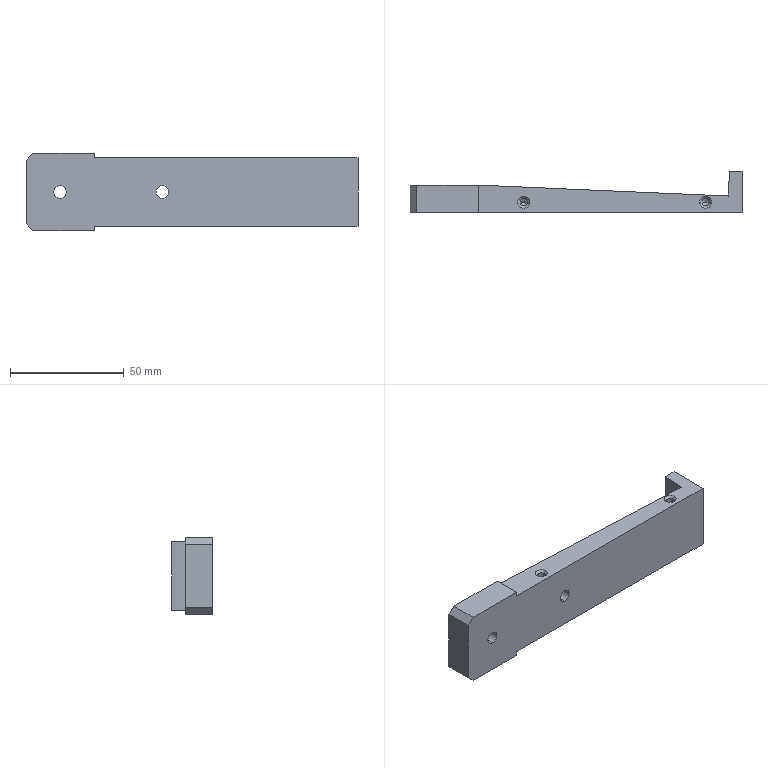Part | SolidWorks | features ICE 4, HoleWzd 3, Chamfer 2, Extrusion 1, MirrorPattern 1 | 1 solid | 57 faces | box 146 x 18 x 34 mm | volume 45286 mm3 | cone 20 | cylinder 20 | plane 17 | commonest cylinder face diameters 3.3 x12 5.5 x4 10 x4
STEP:
#1=CARTESIAN_POINT('',(-24.65,-1.5,14.));
#2=VERTEX_POINT('',#1);
#3=CARTESIAN_POINT('',(-21.35,-1.5,14.));
#4=VERTEX_POINT('',#3);
#5=CARTESIAN_POINT('',(-23.,-1.5,14.));
#6=DIRECTION('',(0.,0.,1.));
#7=DIRECTION('',(-1.,0.,0.));
#8=AXIS2_PLACEMENT_3D('',#5,#6,#7);
#9=CIRCLE('',#8,1.65);
#10=EDGE_CURVE('',#2,#4,#9,.T.);
#11=ORIENTED_EDGE('',*,*,#10,.F.);
#12=CARTESIAN_POINT('',(-25.65,-1.5,15.));
#13=VERTEX_POINT('',#12);
#14=CARTESIAN_POINT('',(-24.65,-1.5,14.));
#15=DIRECTION('',(-0.7071,0.,0.7071));
#16=VECTOR('',#15,1000.);
#17=LINE('',#14,#16);
#18=EDGE_CURVE('',#2,#13,#17,.T.);
#19=ORIENTED_EDGE('',*,*,#18,.T.);
#20=CARTESIAN_POINT('',(-20.35,-1.5,15.));
#21=VERTEX_POINT('',#20);
#22=CARTESIAN_POINT('',(-23.,-1.5,15.));
#23=DIRECTION('',(0.,0.,-1.));
#24=DIRECTION('',(-1.,0.,0.));
#25=AXIS2_PLACEMENT_3D('',#22,#23,#24);
#26=CIRCLE('',#25,2.65);
#27=EDGE_CURVE('',#21,#13,#26,.T.);
#28=ORIENTED_EDGE('',*,*,#27,.F.);
#29=CARTESIAN_POINT('',(-21.35,-1.5,14.));
#30=DIRECTION('',(0.7071,0.,0.7071));
#31=VECTOR('',#30,1000.);
#32=LINE('',#29,#31);
#33=EDGE_CURVE('',#4,#21,#32,.T.);
#34=ORIENTED_EDGE('',*,*,#33,.F.);
#35=EDGE_LOOP('',(#11,#19,#28,#34));
#36=FACE_OUTER_BOUND('',#35,.T.);
#37=CARTESIAN_POINT('',(-23.,-1.5,14.));
#38=DIRECTION('',(0.,0.,1.));
#39=DIRECTION('',(1.,0.,0.));
#40=AXIS2_PLACEMENT_3D('',#37,#38,#39);
#41=CONICAL_SURFACE('',#40,1.65,0.7854);
#42=ADVANCED_FACE('',(#36),#41,.F.);
#43=CARTESIAN_POINT('',(55.35,-1.5,14.));
#44=VERTEX_POINT('',#43);
#45=CARTESIAN_POINT('',(58.65,-1.5,14.));
#46=VERTEX_POINT('',#45);
#47=CARTESIAN_POINT('',(57.,-1.5,14.));
#48=DIRECTION('',(0.,0.,1.));
#49=DIRECTION('',(-1.,0.,0.));
#50=AXIS2_PLACEMENT_3D('',#47,#48,#49);
#51=CIRCLE('',#50,1.65);
#52=EDGE_CURVE('',#44,#46,#51,.T.);
#53=ORIENTED_EDGE('',*,*,#52,.F.);
#54=CARTESIAN_POINT('',(54.35,-1.5,15.));
#55=VERTEX_POINT('',#54);
#56=CARTESIAN_POINT('',(55.35,-1.5,14.));
#57=DIRECTION('',(-0.7071,0.,0.7071));
#58=VECTOR('',#57,1000.);
#59=LINE('',#56,#58);
#60=EDGE_CURVE('',#44,#55,#59,.T.);
#61=ORIENTED_EDGE('',*,*,#60,.T.);
#62=CARTESIAN_POINT('',(59.65,-1.5,15.));
#63=VERTEX_POINT('',#62);
#64=CARTESIAN_POINT('',(57.,-1.5,15.));
#65=DIRECTION('',(0.,0.,-1.));
#66=DIRECTION('',(-1.,0.,0.));
#67=AXIS2_PLACEMENT_3D('',#64,#65,#66);
#68=CIRCLE('',#67,2.65);
#69=EDGE_CURVE('',#63,#55,#68,.T.);
#70=ORIENTED_EDGE('',*,*,#69,.F.);
#71=CARTESIAN_POINT('',(58.65,-1.5,14.));
#72=DIRECTION('',(0.7071,0.,0.7071));
#73=VECTOR('',#72,1000.);
#74=LINE('',#71,#73);
#75=EDGE_CURVE('',#46,#63,#74,.T.);
#76=ORIENTED_EDGE('',*,*,#75,.F.);
#77=EDGE_LOOP('',(#53,#61,#70,#76));
#78=FACE_OUTER_BOUND('',#77,.T.);
#79=CARTESIAN_POINT('',(57.,-1.5,14.));
#80=DIRECTION('',(0.,0.,1.));
#81=DIRECTION('',(1.,0.,0.));
#82=AXIS2_PLACEMENT_3D('',#79,#80,#81);
#83=CONICAL_SURFACE('',#82,1.65,0.7854);
#84=ADVANCED_FACE('',(#78),#83,.F.);
#85=CARTESIAN_POINT('',(58.65,-1.5,-14.));
#86=VERTEX_POINT('',#85);
#87=CARTESIAN_POINT('',(55.35,-1.5,-14.));
#88=VERTEX_POINT('',#87);
#89=CARTESIAN_POINT('',(57.,-1.5,-14.));
#90=DIRECTION('',(0.,0.,-1.));
#91=DIRECTION('',(1.,0.,0.));
#92=AXIS2_PLACEMENT_3D('',#89,#90,#91);
#93=CIRCLE('',#92,1.65);
#94=EDGE_CURVE('',#86,#88,#93,.T.);
#95=ORIENTED_EDGE('',*,*,#94,.F.);
#96=CARTESIAN_POINT('',(59.65,-1.5,-15.));
#97=VERTEX_POINT('',#96);
#98=CARTESIAN_POINT('',(58.65,-1.5,-14.));
#99=DIRECTION('',(0.7071,0.,-0.7071));
#100=VECTOR('',#99,1000.);
#101=LINE('',#98,#100);
#102=EDGE_CURVE('',#86,#97,#101,.T.);
#103=ORIENTED_EDGE('',*,*,#102,.T.);
#104=CARTESIAN_POINT('',(54.35,-1.5,-15.));
#105=VERTEX_POINT('',#104);
#106=CARTESIAN_POINT('',(57.,-1.5,-15.));
#107=DIRECTION('',(0.,0.,1.));
#108=DIRECTION('',(1.,0.,0.));
#109=AXIS2_PLACEMENT_3D('',#106,#107,#108);
#110=CIRCLE('',#109,2.65);
#111=EDGE_CURVE('',#105,#97,#110,.T.);
#112=ORIENTED_EDGE('',*,*,#111,.F.);
#113=CARTESIAN_POINT('',(55.35,-1.5,-14.));
#114=DIRECTION('',(-0.7071,0.,-0.7071));
#115=VECTOR('',#114,1000.);
#116=LINE('',#113,#115);
#117=EDGE_CURVE('',#88,#105,#116,.T.);
#118=ORIENTED_EDGE('',*,*,#117,.F.);
#119=EDGE_LOOP('',(#95,#103,#112,#118));
#120=FACE_OUTER_BOUND('',#119,.T.);
#121=CARTESIAN_POINT('',(57.,-1.5,-14.));
#122=DIRECTION('',(0.,0.,-1.));
#123=DIRECTION('',(-1.,0.,0.));
#124=AXIS2_PLACEMENT_3D('',#121,#122,#123);
#125=CONICAL_SURFACE('',#124,1.65,0.7854);
#126=ADVANCED_FACE('',(#120),#125,.F.);
#127=CARTESIAN_POINT('',(-21.35,-1.5,-14.));
#128=VERTEX_POINT('',#127);
#129=CARTESIAN_POINT('',(-24.65,-1.5,-14.));
#130=VERTEX_POINT('',#129);
#131=CARTESIAN_POINT('',(-23.,-1.5,-14.));
#132=DIRECTION('',(0.,0.,-1.));
#133=DIRECTION('',(1.,0.,0.));
#134=AXIS2_PLACEMENT_3D('',#131,#132,#133);
#135=CIRCLE('',#134,1.65);
#136=EDGE_CURVE('',#128,#130,#135,.T.);
#137=ORIENTED_EDGE('',*,*,#136,.F.);
#138=CARTESIAN_POINT('',(-20.35,-1.5,-15.));
#139=VERTEX_POINT('',#138);
#140=CARTESIAN_POINT('',(-21.35,-1.5,-14.));
#141=DIRECTION('',(0.7071,0.,-0.7071));
#142=VECTOR('',#141,1000.);
#143=LINE('',#140,#142);
#144=EDGE_CURVE('',#128,#139,#143,.T.);
#145=ORIENTED_EDGE('',*,*,#144,.T.);
#146=CARTESIAN_POINT('',(-25.65,-1.5,-15.));
#147=VERTEX_POINT('',#146);
#148=CARTESIAN_POINT('',(-23.,-1.5,-15.));
#149=DIRECTION('',(0.,0.,1.));
#150=DIRECTION('',(1.,0.,0.));
#151=AXIS2_PLACEMENT_3D('',#148,#149,#150);
#152=CIRCLE('',#151,2.65);
#153=EDGE_CURVE('',#147,#139,#152,.T.);
#154=ORIENTED_EDGE('',*,*,#153,.F.);
#155=CARTESIAN_POINT('',(-24.65,-1.5,-14.));
#156=DIRECTION('',(-0.7071,0.,-0.7071));
#157=VECTOR('',#156,1000.);
#158=LINE('',#155,#157);
#159=EDGE_CURVE('',#130,#147,#158,.T.);
#160=ORIENTED_EDGE('',*,*,#159,.F.);
#161=EDGE_LOOP('',(#137,#145,#154,#160));
#162=FACE_OUTER_BOUND('',#161,.T.);
#163=CARTESIAN_POINT('',(-23.,-1.5,-14.));
#164=DIRECTION('',(0.,0.,-1.));
#165=DIRECTION('',(-1.,0.,0.));
#166=AXIS2_PLACEMENT_3D('',#163,#164,#165);
#167=CONICAL_SURFACE('',#166,1.65,0.7854);
#168=ADVANCED_FACE('',(#162),#167,.F.);
#169=CARTESIAN_POINT('',(-21.35,-1.5,-4.9));
#170=VERTEX_POINT('',#169);
#171=CARTESIAN_POINT('',(-24.65,-1.5,-4.9));
#172=VERTEX_POINT('',#171);
#173=CARTESIAN_POINT('',(-23.,-1.5,-4.9));
#174=DIRECTION('',(0.,0.,-1.));
#175=DIRECTION('',(-1.,0.,0.));
#176=AXIS2_PLACEMENT_3D('',#173,#174,#175);
#177=CIRCLE('',#176,1.65);
#178=EDGE_CURVE('',#170,#172,#177,.T.);
#179=ORIENTED_EDGE('',*,*,#178,.F.);
#180=CARTESIAN_POINT('',(-21.35,-1.5,-15.));
#181=DIRECTION('',(0.,0.,-1.));
#182=VECTOR('',#181,1000.);
#183=LINE('',#180,#182);
#184=EDGE_CURVE('',#170,#128,#183,.T.);
#185=ORIENTED_EDGE('',*,*,#184,.T.);
#186=ORIENTED_EDGE('',*,*,#136,.T.);
#187=CARTESIAN_POINT('',(-24.65,-1.5,-15.));
#188=DIRECTION('',(0.,0.,-1.));
#189=VECTOR('',#188,1000.);
#190=LINE('',#187,#189);
#191=EDGE_CURVE('',#172,#130,#190,.T.);
#192=ORIENTED_EDGE('',*,*,#191,.F.);
#193=EDGE_LOOP('',(#179,#185,#186,#192));
#194=FACE_OUTER_BOUND('',#193,.T.);
#195=CARTESIAN_POINT('',(-23.,-1.5,-15.));
#196=DIRECTION('',(0.,0.,-1.));
#197=DIRECTION('',(-1.,0.,0.));
#198=AXIS2_PLACEMENT_3D('',#195,#196,#197);
#199=CYLINDRICAL_SURFACE('',#198,1.65);
#200=ADVANCED_FACE('',(#194),#199,.F.);
#201=CARTESIAN_POINT('',(-23.,-1.5,-3.909));
#202=VERTEX_POINT('',#201);
#203=CARTESIAN_POINT('',(-24.65,-1.5,-4.9));
#204=DIRECTION('',(-0.8572,0.,-0.515));
#205=VECTOR('',#204,1000.);
#206=LINE('',#203,#205);
#207=EDGE_CURVE('',#202,#172,#206,.T.);
#208=ORIENTED_EDGE('',*,*,#207,.F.);
#209=CARTESIAN_POINT('',(-21.35,-1.5,-4.9));
#210=DIRECTION('',(0.8572,0.,-0.515));
#211=VECTOR('',#210,1000.);
#212=LINE('',#209,#211);
#213=EDGE_CURVE('',#202,#170,#212,.T.);
#214=ORIENTED_EDGE('',*,*,#213,.T.);
#215=ORIENTED_EDGE('',*,*,#178,.T.);
#216=EDGE_LOOP('',(#208,#214,#215));
#217=FACE_OUTER_BOUND('',#216,.T.);
#218=CARTESIAN_POINT('',(-23.,-1.5,-4.9));
#219=DIRECTION('',(0.,0.,-1.));
#220=DIRECTION('',(-1.,0.,0.));
#221=AXIS2_PLACEMENT_3D('',#218,#219,#220);
#222=CONICAL_SURFACE('',#221,1.65,1.03);
#223=ADVANCED_FACE('',(#217),#222,.F.);
#224=CARTESIAN_POINT('',(58.65,-1.5,-4.9));
#225=VERTEX_POINT('',#224);
#226=CARTESIAN_POINT('',(55.35,-1.5,-4.9));
#227=VERTEX_POINT('',#226);
#228=CARTESIAN_POINT('',(57.,-1.5,-4.9));
#229=DIRECTION('',(0.,0.,-1.));
#230=DIRECTION('',(-1.,0.,0.));
#231=AXIS2_PLACEMENT_3D('',#228,#229,#230);
#232=CIRCLE('',#231,1.65);
#233=EDGE_CURVE('',#225,#227,#232,.T.);
#234=ORIENTED_EDGE('',*,*,#233,.F.);
#235=CARTESIAN_POINT('',(58.65,-1.5,-15.));
#236=DIRECTION('',(0.,0.,-1.));
#237=VECTOR('',#236,1000.);
#238=LINE('',#235,#237);
#239=EDGE_CURVE('',#225,#86,#238,.T.);
#240=ORIENTED_EDGE('',*,*,#239,.T.);
#241=ORIENTED_EDGE('',*,*,#94,.T.);
#242=CARTESIAN_POINT('',(55.35,-1.5,-15.));
#243=DIRECTION('',(0.,0.,-1.));
#244=VECTOR('',#243,1000.);
#245=LINE('',#242,#244);
#246=EDGE_CURVE('',#227,#88,#245,.T.);
#247=ORIENTED_EDGE('',*,*,#246,.F.);
#248=EDGE_LOOP('',(#234,#240,#241,#247));
#249=FACE_OUTER_BOUND('',#248,.T.);
#250=CARTESIAN_POINT('',(57.,-1.5,-15.));
#251=DIRECTION('',(0.,0.,-1.));
#252=DIRECTION('',(-1.,0.,0.));
#253=AXIS2_PLACEMENT_3D('',#250,#251,#252);
#254=CYLINDRICAL_SURFACE('',#253,1.65);
#255=ADVANCED_FACE('',(#249),#254,.F.);
#256=CARTESIAN_POINT('',(57.,-1.5,-3.909));
#257=VERTEX_POINT('',#256);
#258=CARTESIAN_POINT('',(55.35,-1.5,-4.9));
#259=DIRECTION('',(-0.8572,0.,-0.515));
#260=VECTOR('',#259,1000.);
#261=LINE('',#258,#260);
#262=EDGE_CURVE('',#257,#227,#261,.T.);
#263=ORIENTED_EDGE('',*,*,#262,.F.);
#264=CARTESIAN_POINT('',(58.65,-1.5,-4.9));
#265=DIRECTION('',(0.8572,0.,-0.515));
#266=VECTOR('',#265,1000.);
#267=LINE('',#264,#266);
#268=EDGE_CURVE('',#257,#225,#267,.T.);
#269=ORIENTED_EDGE('',*,*,#268,.T.);
#270=ORIENTED_EDGE('',*,*,#233,.T.);
#271=EDGE_LOOP('',(#263,#269,#270));
#272=FACE_OUTER_BOUND('',#271,.T.);
#273=CARTESIAN_POINT('',(57.,-1.5,-4.9));
#274=DIRECTION('',(0.,0.,-1.));
#275=DIRECTION('',(-1.,0.,0.));
#276=AXIS2_PLACEMENT_3D('',#273,#274,#275);
#277=CONICAL_SURFACE('',#276,1.65,1.03);
#278=ADVANCED_FACE('',(#272),#277,.F.);
#279=CARTESIAN_POINT('',(-24.65,-1.5,4.9));
#280=VERTEX_POINT('',#279);
#281=CARTESIAN_POINT('',(-21.35,-1.5,4.9));
#282=VERTEX_POINT('',#281);
#283=CARTESIAN_POINT('',(-23.,-1.5,4.9));
#284=DIRECTION('',(0.,0.,1.));
#285=DIRECTION('',(1.,0.,0.));
#286=AXIS2_PLACEMENT_3D('',#283,#284,#285);
#287=CIRCLE('',#286,1.65);
#288=EDGE_CURVE('',#280,#282,#287,.T.);
#289=ORIENTED_EDGE('',*,*,#288,.F.);
#290=CARTESIAN_POINT('',(-24.65,-1.5,15.));
#291=DIRECTION('',(0.,0.,1.));
#292=VECTOR('',#291,1000.);
#293=LINE('',#290,#292);
#294=EDGE_CURVE('',#280,#2,#293,.T.);
#295=ORIENTED_EDGE('',*,*,#294,.T.);
#296=ORIENTED_EDGE('',*,*,#10,.T.);
#297=CARTESIAN_POINT('',(-21.35,-1.5,15.));
#298=DIRECTION('',(0.,0.,1.));
#299=VECTOR('',#298,1000.);
#300=LINE('',#297,#299);
#301=EDGE_CURVE('',#282,#4,#300,.T.);
#302=ORIENTED_EDGE('',*,*,#301,.F.);
#303=EDGE_LOOP('',(#289,#295,#296,#302));
#304=FACE_OUTER_BOUND('',#303,.T.);
#305=CARTESIAN_POINT('',(-23.,-1.5,15.));
#306=DIRECTION('',(0.,0.,1.));
#307=DIRECTION('',(1.,0.,0.));
#308=AXIS2_PLACEMENT_3D('',#305,#306,#307);
#309=CYLINDRICAL_SURFACE('',#308,1.65);
#310=ADVANCED_FACE('',(#304),#309,.F.);
#311=CARTESIAN_POINT('',(-23.,-1.5,3.909));
#312=VERTEX_POINT('',#311);
#313=CARTESIAN_POINT('',(-21.35,-1.5,4.9));
#314=DIRECTION('',(0.8572,0.,0.515));
#315=VECTOR('',#314,1000.);
#316=LINE('',#313,#315);
#317=EDGE_CURVE('',#312,#282,#316,.T.);
#318=ORIENTED_EDGE('',*,*,#317,.F.);
#319=CARTESIAN_POINT('',(-24.65,-1.5,4.9));
#320=DIRECTION('',(-0.8572,0.,0.515));
#321=VECTOR('',#320,1000.);
#322=LINE('',#319,#321);
#323=EDGE_CURVE('',#312,#280,#322,.T.);
#324=ORIENTED_EDGE('',*,*,#323,.T.);
#325=ORIENTED_EDGE('',*,*,#288,.T.);
#326=EDGE_LOOP('',(#318,#324,#325));
#327=FACE_OUTER_BOUND('',#326,.T.);
#328=CARTESIAN_POINT('',(-23.,-1.5,4.9));
#329=DIRECTION('',(0.,0.,1.));
#330=DIRECTION('',(1.,0.,0.));
#331=AXIS2_PLACEMENT_3D('',#328,#329,#330);
#332=CONICAL_SURFACE('',#331,1.65,1.03);
#333=ADVANCED_FACE('',(#327),#332,.F.);
#334=CARTESIAN_POINT('',(55.35,-1.5,4.9));
#335=VERTEX_POINT('',#334);
#336=CARTESIAN_POINT('',(58.65,-1.5,4.9));
#337=VERTEX_POINT('',#336);
#338=CARTESIAN_POINT('',(57.,-1.5,4.9));
#339=DIRECTION('',(0.,0.,1.));
#340=DIRECTION('',(1.,0.,0.));
#341=AXIS2_PLACEMENT_3D('',#338,#339,#340);
#342=CIRCLE('',#341,1.65);
#343=EDGE_CURVE('',#335,#337,#342,.T.);
#344=ORIENTED_EDGE('',*,*,#343,.F.);
#345=CARTESIAN_POINT('',(55.35,-1.5,15.));
#346=DIRECTION('',(0.,0.,1.));
#347=VECTOR('',#346,1000.);
#348=LINE('',#345,#347);
#349=EDGE_CURVE('',#335,#44,#348,.T.);
#350=ORIENTED_EDGE('',*,*,#349,.T.);
#351=ORIENTED_EDGE('',*,*,#52,.T.);
#352=CARTESIAN_POINT('',(58.65,-1.5,15.));
#353=DIRECTION('',(0.,0.,1.));
#354=VECTOR('',#353,1000.);
#355=LINE('',#352,#354);
#356=EDGE_CURVE('',#337,#46,#355,.T.);
#357=ORIENTED_EDGE('',*,*,#356,.F.);
#358=EDGE_LOOP('',(#344,#350,#351,#357));
#359=FACE_OUTER_BOUND('',#358,.T.);
#360=CARTESIAN_POINT('',(57.,-1.5,15.));
#361=DIRECTION('',(0.,0.,1.));
#362=DIRECTION('',(1.,0.,0.));
#363=AXIS2_PLACEMENT_3D('',#360,#361,#362);
#364=CYLINDRICAL_SURFACE('',#363,1.65);
#365=ADVANCED_FACE('',(#359),#364,.F.);
#366=CARTESIAN_POINT('',(57.,-1.5,3.909));
#367=VERTEX_POINT('',#366);
#368=CARTESIAN_POINT('',(58.65,-1.5,4.9));
#369=DIRECTION('',(0.8572,0.,0.515));
#370=VECTOR('',#369,1000.);
#371=LINE('',#368,#370);
#372=EDGE_CURVE('',#367,#337,#371,.T.);
#373=ORIENTED_EDGE('',*,*,#372,.F.);
#374=CARTESIAN_POINT('',(55.35,-1.5,4.9));
#375=DIRECTION('',(-0.8572,0.,0.515));
#376=VECTOR('',#375,1000.);
#377=LINE('',#374,#376);
#378=EDGE_CURVE('',#367,#335,#377,.T.);
#379=ORIENTED_EDGE('',*,*,#378,.T.);
#380=ORIENTED_EDGE('',*,*,#343,.T.);
#381=EDGE_LOOP('',(#373,#379,#380));
#382=FACE_OUTER_BOUND('',#381,.T.);
#383=CARTESIAN_POINT('',(57.,-1.5,4.9));
#384=DIRECTION('',(0.,0.,1.));
#385=DIRECTION('',(1.,0.,0.));
#386=AXIS2_PLACEMENT_3D('',#383,#384,#385);
#387=CONICAL_SURFACE('',#386,1.65,1.03);
#388=ADVANCED_FACE('',(#382),#387,.F.);
#389=CARTESIAN_POINT('',(62.9,-1.5,11.65));
#390=VERTEX_POINT('',#389);
#391=CARTESIAN_POINT('',(62.9,-1.5,8.35));
#392=VERTEX_POINT('',#391);
#393=CARTESIAN_POINT('',(62.9,-1.5,10.));
#394=DIRECTION('',(1.,0.,0.));
#395=DIRECTION('',(0.,0.,-1.));
#396=AXIS2_PLACEMENT_3D('',#393,#394,#395);
#397=CIRCLE('',#396,1.65);
#398=EDGE_CURVE('',#390,#392,#397,.T.);
#399=ORIENTED_EDGE('',*,*,#398,.F.);
#400=CARTESIAN_POINT('',(73.,-1.5,11.65));
#401=VERTEX_POINT('',#400);
#402=CARTESIAN_POINT('',(73.,-1.5,11.65));
#403=DIRECTION('',(1.,0.,0.));
#404=VECTOR('',#403,1000.);
#405=LINE('',#402,#404);
#406=EDGE_CURVE('',#390,#401,#405,.T.);
#407=ORIENTED_EDGE('',*,*,#406,.T.);
#408=CARTESIAN_POINT('',(73.,-1.5,8.35));
#409=VERTEX_POINT('',#408);
#410=CARTESIAN_POINT('',(73.,-1.5,10.));
#411=DIRECTION('',(1.,0.,0.));
#412=DIRECTION('',(0.,0.,-1.));
#413=AXIS2_PLACEMENT_3D('',#410,#411,#412);
#414=CIRCLE('',#413,1.65);
#415=EDGE_CURVE('',#401,#409,#414,.T.);
#416=ORIENTED_EDGE('',*,*,#415,.T.);
#417=CARTESIAN_POINT('',(73.,-1.5,8.35));
#418=DIRECTION('',(1.,0.,0.));
#419=VECTOR('',#418,1000.);
#420=LINE('',#417,#419);
#421=EDGE_CURVE('',#392,#409,#420,.T.);
#422=ORIENTED_EDGE('',*,*,#421,.F.);
#423=EDGE_LOOP('',(#399,#407,#416,#422));
#424=FACE_OUTER_BOUND('',#423,.T.);
#425=CARTESIAN_POINT('',(73.,-1.5,10.));
#426=DIRECTION('',(1.,0.,0.));
#427=DIRECTION('',(0.,0.,-1.));
#428=AXIS2_PLACEMENT_3D('',#425,#426,#427);
#429=CYLINDRICAL_SURFACE('',#428,1.65);
#430=ADVANCED_FACE('',(#424),#429,.F.);
#431=CARTESIAN_POINT('',(61.909,-1.5,10.));
#432=VERTEX_POINT('',#431);
#433=CARTESIAN_POINT('',(62.9,-1.5,8.35));
#434=DIRECTION('',(0.515,0.,-0.8572));
#435=VECTOR('',#434,1000.);
#436=LINE('',#433,#435);
#437=EDGE_CURVE('',#432,#392,#436,.T.);
#438=ORIENTED_EDGE('',*,*,#437,.F.);
#439=CARTESIAN_POINT('',(62.9,-1.5,11.65));
#440=DIRECTION('',(0.515,0.,0.8572));
#441=VECTOR('',#440,1000.);
#442=LINE('',#439,#441);
#443=EDGE_CURVE('',#432,#390,#442,.T.);
#444=ORIENTED_EDGE('',*,*,#443,.T.);
#445=ORIENTED_EDGE('',*,*,#398,.T.);
#446=EDGE_LOOP('',(#438,#444,#445));
#447=FACE_OUTER_BOUND('',#446,.T.);
#448=CARTESIAN_POINT('',(62.9,-1.5,10.));
#449=DIRECTION('',(1.,0.,0.));
#450=DIRECTION('',(0.,0.,-1.));
#451=AXIS2_PLACEMENT_3D('',#448,#449,#450);
#452=CONICAL_SURFACE('',#451,1.65,1.03);
#453=ADVANCED_FACE('',(#447),#452,.F.);
#454=CARTESIAN_POINT('',(62.9,-1.5,-8.35));
#455=VERTEX_POINT('',#454);
#456=CARTESIAN_POINT('',(62.9,-1.5,-11.65));
#457=VERTEX_POINT('',#456);
#458=CARTESIAN_POINT('',(62.9,-1.5,-10.));
#459=DIRECTION('',(1.,0.,0.));
#460=DIRECTION('',(0.,0.,-1.));
#461=AXIS2_PLACEMENT_3D('',#458,#459,#460);
#462=CIRCLE('',#461,1.65);
#463=EDGE_CURVE('',#455,#457,#462,.T.);
#464=ORIENTED_EDGE('',*,*,#463,.F.);
#465=CARTESIAN_POINT('',(73.,-1.5,-8.35));
#466=VERTEX_POINT('',#465);
#467=CARTESIAN_POINT('',(73.,-1.5,-8.35));
#468=DIRECTION('',(1.,0.,0.));
#469=VECTOR('',#468,1000.);
#470=LINE('',#467,#469);
#471=EDGE_CURVE('',#455,#466,#470,.T.);
#472=ORIENTED_EDGE('',*,*,#471,.T.);
#473=CARTESIAN_POINT('',(73.,-1.5,-11.65));
#474=VERTEX_POINT('',#473);
#475=CARTESIAN_POINT('',(73.,-1.5,-10.));
#476=DIRECTION('',(1.,0.,0.));
#477=DIRECTION('',(0.,0.,-1.));
#478=AXIS2_PLACEMENT_3D('',#475,#476,#477);
#479=CIRCLE('',#478,1.65);
#480=EDGE_CURVE('',#466,#474,#479,.T.);
#481=ORIENTED_EDGE('',*,*,#480,.T.);
#482=CARTESIAN_POINT('',(73.,-1.5,-11.65));
#483=DIRECTION('',(1.,0.,0.));
#484=VECTOR('',#483,1000.);
#485=LINE('',#482,#484);
#486=EDGE_CURVE('',#457,#474,#485,.T.);
#487=ORIENTED_EDGE('',*,*,#486,.F.);
#488=EDGE_LOOP('',(#464,#472,#481,#487));
#489=FACE_OUTER_BOUND('',#488,.T.);
#490=CARTESIAN_POINT('',(73.,-1.5,-10.));
#491=DIRECTION('',(1.,0.,0.));
#492=DIRECTION('',(0.,0.,-1.));
#493=AXIS2_PLACEMENT_3D('',#490,#491,#492);
#494=CYLINDRICAL_SURFACE('',#493,1.65);
#495=ADVANCED_FACE('',(#489),#494,.F.);
#496=CARTESIAN_POINT('',(61.909,-1.5,-10.));
#497=VERTEX_POINT('',#496);
#498=CARTESIAN_POINT('',(62.9,-1.5,-11.65));
#499=DIRECTION('',(0.515,0.,-0.8572));
#500=VECTOR('',#499,1000.);
#501=LINE('',#498,#500);
#502=EDGE_CURVE('',#497,#457,#501,.T.);
#503=ORIENTED_EDGE('',*,*,#502,.F.);
#504=CARTESIAN_POINT('',(62.9,-1.5,-8.35));
#505=DIRECTION('',(0.515,0.,0.8572));
#506=VECTOR('',#505,1000.);
#507=LINE('',#504,#506);
#508=EDGE_CURVE('',#497,#455,#507,.T.);
#509=ORIENTED_EDGE('',*,*,#508,.T.);
#510=ORIENTED_EDGE('',*,*,#463,.T.);
#511=EDGE_LOOP('',(#503,#509,#510));
#512=FACE_OUTER_BOUND('',#511,.T.);
#513=CARTESIAN_POINT('',(62.9,-1.5,-10.));
#514=DIRECTION('',(1.,0.,0.));
#515=DIRECTION('',(0.,0.,-1.));
#516=AXIS2_PLACEMENT_3D('',#513,#514,#515);
#517=CONICAL_SURFACE('',#516,1.65,1.03);
#518=ADVANCED_FACE('',(#512),#517,.F.);
#519=CARTESIAN_POINT('',(-58.,0.,-5.));
#520=VERTEX_POINT('',#519);
#521=CARTESIAN_POINT('',(-58.,0.,5.));
#522=VERTEX_POINT('',#521);
#523=CARTESIAN_POINT('',(-58.,0.,0.));
#524=DIRECTION('',(0.,1.,0.));
#525=DIRECTION('',(0.,0.,1.));
#526=AXIS2_PLACEMENT_3D('',#523,#524,#525);
#527=CIRCLE('',#526,5.);
#528=EDGE_CURVE('',#520,#522,#527,.T.);
#529=ORIENTED_EDGE('',*,*,#528,.F.);
#530=CARTESIAN_POINT('',(-58.,6.,-5.));
#531=VERTEX_POINT('',#530);
#532=CARTESIAN_POINT('',(-58.,6.,-5.));
#533=DIRECTION('',(0.,1.,0.));
#534=VECTOR('',#533,1000.);
#535=LINE('',#532,#534);
#536=EDGE_CURVE('',#520,#531,#535,.T.);
#537=ORIENTED_EDGE('',*,*,#536,.T.);
#538=CARTESIAN_POINT('',(-58.,6.,5.));
#539=VERTEX_POINT('',#538);
#540=CARTESIAN_POINT('',(-58.,6.,0.));
#541=DIRECTION('',(0.,1.,0.));
#542=DIRECTION('',(0.,0.,1.));
#543=AXIS2_PLACEMENT_3D('',#540,#541,#542);
#544=CIRCLE('',#543,5.);
#545=EDGE_CURVE('',#531,#539,#544,.T.);
#546=ORIENTED_EDGE('',*,*,#545,.T.);
#547=CARTESIAN_POINT('',(-58.,6.,5.));
#548=DIRECTION('',(0.,1.,0.));
#549=VECTOR('',#548,1000.);
#550=LINE('',#547,#549);
#551=EDGE_CURVE('',#522,#539,#550,.T.);
#552=ORIENTED_EDGE('',*,*,#551,.F.);
#553=EDGE_LOOP('',(#529,#537,#546,#552));
#554=FACE_OUTER_BOUND('',#553,.T.);
#555=CARTESIAN_POINT('',(-58.,6.,0.));
#556=DIRECTION('',(0.,1.,0.));
#557=DIRECTION('',(0.,0.,1.));
#558=AXIS2_PLACEMENT_3D('',#555,#556,#557);
#559=CYLINDRICAL_SURFACE('',#558,5.);
#560=ADVANCED_FACE('',(#554),#559,.F.);
#561=CARTESIAN_POINT('',(-58.,-6.,-2.75));
#562=VERTEX_POINT('',#561);
#563=CARTESIAN_POINT('',(-58.,-6.,2.75));
#564=VERTEX_POINT('',#563);
#565=CARTESIAN_POINT('',(-58.,-6.,0.));
#566=DIRECTION('',(0.,1.,0.));
#567=DIRECTION('',(0.,0.,1.));
#568=AXIS2_PLACEMENT_3D('',#565,#566,#567);
#569=CIRCLE('',#568,2.75);
#570=EDGE_CURVE('',#562,#564,#569,.T.);
#571=ORIENTED_EDGE('',*,*,#570,.F.);
#572=CARTESIAN_POINT('',(-58.,0.,-2.75));
#573=VERTEX_POINT('',#572);
#574=CARTESIAN_POINT('',(-58.,6.,-2.75));
#575=DIRECTION('',(0.,1.,0.));
#576=VECTOR('',#575,1000.);
#577=LINE('',#574,#576);
#578=EDGE_CURVE('',#562,#573,#577,.T.);
#579=ORIENTED_EDGE('',*,*,#578,.T.);
#580=CARTESIAN_POINT('',(-58.,0.,2.75));
#581=VERTEX_POINT('',#580);
#582=CARTESIAN_POINT('',(-58.,0.,0.));
#583=DIRECTION('',(0.,1.,0.));
#584=DIRECTION('',(0.,0.,1.));
#585=AXIS2_PLACEMENT_3D('',#582,#583,#584);
#586=CIRCLE('',#585,2.75);
#587=EDGE_CURVE('',#573,#581,#586,.T.);
#588=ORIENTED_EDGE('',*,*,#587,.T.);
#589=CARTESIAN_POINT('',(-58.,6.,2.75));
#590=DIRECTION('',(0.,1.,0.));
#591=VECTOR('',#590,1000.);
#592=LINE('',#589,#591);
#593=EDGE_CURVE('',#564,#581,#592,.T.);
#594=ORIENTED_EDGE('',*,*,#593,.F.);
#595=EDGE_LOOP('',(#571,#579,#588,#594));
#596=FACE_OUTER_BOUND('',#595,.T.);
#597=CARTESIAN_POINT('',(-58.,6.,0.));
#598=DIRECTION('',(0.,1.,0.));
#599=DIRECTION('',(0.,0.,1.));
#600=AXIS2_PLACEMENT_3D('',#597,#598,#599);
#601=CYLINDRICAL_SURFACE('',#600,2.75);
#602=ADVANCED_FACE('',(#596),#601,.F.);
#603=CARTESIAN_POINT('',(-13.,0.,-5.));
#604=VERTEX_POINT('',#603);
#605=CARTESIAN_POINT('',(-13.,0.,5.));
#606=VERTEX_POINT('',#605);
#607=CARTESIAN_POINT('',(-13.,0.,0.));
#608=DIRECTION('',(0.,1.,0.));
#609=DIRECTION('',(0.,0.,1.));
#610=AXIS2_PLACEMENT_3D('',#607,#608,#609);
#611=CIRCLE('',#610,5.);
#612=EDGE_CURVE('',#604,#606,#611,.T.);
#613=ORIENTED_EDGE('',*,*,#612,.F.);
#614=CARTESIAN_POINT('',(-13.,4.69,-5.));
#615=VERTEX_POINT('',#614);
#616=CARTESIAN_POINT('',(-13.,6.,-5.));
#617=DIRECTION('',(0.,1.,0.));
#618=VECTOR('',#617,1000.);
#619=LINE('',#616,#618);
#620=EDGE_CURVE('',#604,#615,#619,.T.);
#621=ORIENTED_EDGE('',*,*,#620,.T.);
#622=CARTESIAN_POINT('',(-13.,4.69,5.));
#623=VERTEX_POINT('',#622);
#624=CARTESIAN_POINT('',(-13.,4.69,-5.));
#625=CARTESIAN_POINT('',(-23.,5.127,-5.));
#626=CARTESIAN_POINT('',(-23.,5.127,5.));
#627=CARTESIAN_POINT('',(-13.,4.69,5.));
#628=(BOUNDED_CURVE()B_SPLINE_CURVE(3,(#624,#625,#626,#627),.UNSPECIFIED.,.F.,.F.)B_SPLINE_CURVE_WITH_KNOTS((4,4),(4.712,7.854),.UNSPECIFIED.)CURVE()GEOMETRIC_REPRESENTATION_ITEM()RATIONAL_B_SPLINE_CURVE((1.,0.3333,0.3333,1.))REPRESENTATION_ITEM(''));
#629=EDGE_CURVE('',#615,#623,#628,.T.);
#630=ORIENTED_EDGE('',*,*,#629,.T.);
#631=CARTESIAN_POINT('',(-13.,6.,5.));
#632=DIRECTION('',(0.,1.,0.));
#633=VECTOR('',#632,1000.);
#634=LINE('',#631,#633);
#635=EDGE_CURVE('',#606,#623,#634,.T.);
#636=ORIENTED_EDGE('',*,*,#635,.F.);
#637=EDGE_LOOP('',(#613,#621,#630,#636));
#638=FACE_OUTER_BOUND('',#637,.T.);
#639=CARTESIAN_POINT('',(-13.,6.,0.));
#640=DIRECTION('',(0.,1.,0.));
#641=DIRECTION('',(0.,0.,1.));
#642=AXIS2_PLACEMENT_3D('',#639,#640,#641);
#643=CYLINDRICAL_SURFACE('',#642,5.);
#644=ADVANCED_FACE('',(#638),#643,.F.);
#645=CARTESIAN_POINT('',(-13.,-6.,-2.75));
#646=VERTEX_POINT('',#645);
#647=CARTESIAN_POINT('',(-13.,-6.,2.75));
#648=VERTEX_POINT('',#647);
#649=CARTESIAN_POINT('',(-13.,-6.,0.));
#650=DIRECTION('',(0.,1.,0.));
#651=DIRECTION('',(0.,0.,1.));
#652=AXIS2_PLACEMENT_3D('',#649,#650,#651);
#653=CIRCLE('',#652,2.75);
#654=EDGE_CURVE('',#646,#648,#653,.T.);
#655=ORIENTED_EDGE('',*,*,#654,.F.);
#656=CARTESIAN_POINT('',(-13.,0.,-2.75));
#657=VERTEX_POINT('',#656);
#658=CARTESIAN_POINT('',(-13.,6.,-2.75));
#659=DIRECTION('',(0.,1.,0.));
#660=VECTOR('',#659,1000.);
#661=LINE('',#658,#660);
#662=EDGE_CURVE('',#646,#657,#661,.T.);
#663=ORIENTED_EDGE('',*,*,#662,.T.);
#664=CARTESIAN_POINT('',(-13.,0.,2.75));
#665=VERTEX_POINT('',#664);
#666=CARTESIAN_POINT('',(-13.,0.,0.));
#667=DIRECTION('',(0.,1.,0.));
#668=DIRECTION('',(0.,0.,1.));
#669=AXIS2_PLACEMENT_3D('',#666,#667,#668);
#670=CIRCLE('',#669,2.75);
#671=EDGE_CURVE('',#657,#665,#670,.T.);
#672=ORIENTED_EDGE('',*,*,#671,.T.);
#673=CARTESIAN_POINT('',(-13.,6.,2.75));
#674=DIRECTION('',(0.,1.,0.));
#675=VECTOR('',#674,1000.);
#676=LINE('',#673,#675);
#677=EDGE_CURVE('',#648,#665,#676,.T.);
#678=ORIENTED_EDGE('',*,*,#677,.F.);
#679=EDGE_LOOP('',(#655,#663,#672,#678));
#680=FACE_OUTER_BOUND('',#679,.T.);
#681=CARTESIAN_POINT('',(-13.,6.,0.));
#682=DIRECTION('',(0.,1.,0.));
#683=DIRECTION('',(0.,0.,1.));
#684=AXIS2_PLACEMENT_3D('',#681,#682,#683);
#685=CYLINDRICAL_SURFACE('',#684,2.75);
#686=ADVANCED_FACE('',(#680),#685,.F.);
#687=CARTESIAN_POINT('',(73.,-1.5,10.));
#688=DIRECTION('',(1.,0.,0.));
#689=DIRECTION('',(0.,0.,-1.));
#690=AXIS2_PLACEMENT_3D('',#687,#688,#689);
#691=CIRCLE('',#690,1.65);
#692=EDGE_CURVE('',#409,#401,#691,.T.);
#693=ORIENTED_EDGE('',*,*,#692,.F.);
#694=ORIENTED_EDGE('',*,*,#415,.F.);
#695=EDGE_LOOP('',(#693,#694));
#696=FACE_BOUND('',#695,.T.);
#697=CARTESIAN_POINT('',(73.,-1.5,-10.));
#698=DIRECTION('',(1.,0.,0.));
#699=DIRECTION('',(0.,0.,-1.));
#700=AXIS2_PLACEMENT_3D('',#697,#698,#699);
#701=CIRCLE('',#700,1.65);
#702=EDGE_CURVE('',#474,#466,#701,.T.);
#703=ORIENTED_EDGE('',*,*,#702,.F.);
#704=ORIENTED_EDGE('',*,*,#480,.F.);
#705=EDGE_LOOP('',(#703,#704));
#706=FACE_BOUND('',#705,.T.);
#707=CARTESIAN_POINT('',(73.,-6.,15.));
#708=VERTEX_POINT('',#707);
#709=CARTESIAN_POINT('',(73.,-6.,-15.));
#710=VERTEX_POINT('',#709);
#711=CARTESIAN_POINT('',(73.,-6.,-17.));
#712=DIRECTION('',(0.,0.,-1.));
#713=VECTOR('',#712,1000.);
#714=LINE('',#711,#713);
#715=EDGE_CURVE('',#708,#710,#714,.T.);
#716=ORIENTED_EDGE('',*,*,#715,.T.);
#717=CARTESIAN_POINT('',(73.,12.,-15.));
#718=VERTEX_POINT('',#717);
#719=CARTESIAN_POINT('',(73.,-6.,-15.));
#720=DIRECTION('',(0.,1.,0.));
#721=VECTOR('',#720,1000.);
#722=LINE('',#719,#721);
#723=EDGE_CURVE('',#710,#718,#722,.T.);
#724=ORIENTED_EDGE('',*,*,#723,.T.);
#725=CARTESIAN_POINT('',(73.,12.,15.));
#726=VERTEX_POINT('',#725);
#727=CARTESIAN_POINT('',(73.,12.,15.));
#728=DIRECTION('',(0.,0.,-1.));
#729=VECTOR('',#728,1000.);
#730=LINE('',#727,#729);
#731=EDGE_CURVE('',#726,#718,#730,.T.);
#732=ORIENTED_EDGE('',*,*,#731,.F.);
#733=CARTESIAN_POINT('',(73.,-6.,15.));
#734=DIRECTION('',(0.,1.,0.));
#735=VECTOR('',#734,1000.);
#736=LINE('',#733,#735);
#737=EDGE_CURVE('',#708,#726,#736,.T.);
#738=ORIENTED_EDGE('',*,*,#737,.F.);
#739=EDGE_LOOP('',(#716,#724,#732,#738));
#740=FACE_OUTER_BOUND('',#739,.T.);
#741=CARTESIAN_POINT('',(73.,6.,-17.));
#742=DIRECTION('',(-1.,0.,0.));
#743=DIRECTION('',(0.,0.,1.));
#744=AXIS2_PLACEMENT_3D('',#741,#742,#743);
#745=PLANE('',#744);
#746=ADVANCED_FACE('',(#696,#706,#740),#745,.F.);
#747=CARTESIAN_POINT('',(-43.,6.,-17.));
#748=VERTEX_POINT('',#747);
#749=CARTESIAN_POINT('',(-70.,6.,-17.));
#750=VERTEX_POINT('',#749);
#751=CARTESIAN_POINT('',(-73.,6.,-17.));
#752=DIRECTION('',(-1.,0.,0.));
#753=VECTOR('',#752,1000.);
#754=LINE('',#751,#753);
#755=EDGE_CURVE('',#748,#750,#754,.T.);
#756=ORIENTED_EDGE('',*,*,#755,.F.);
#757=CARTESIAN_POINT('',(-43.,-6.,-17.));
#758=VERTEX_POINT('',#757);
#759=CARTESIAN_POINT('',(-43.,-6.,-17.));
#760=DIRECTION('',(0.,1.,0.));
#761=VECTOR('',#760,1000.);
#762=LINE('',#759,#761);
#763=EDGE_CURVE('',#758,#748,#762,.T.);
#764=ORIENTED_EDGE('',*,*,#763,.F.);
#765=CARTESIAN_POINT('',(-70.,-6.,-17.));
#766=VERTEX_POINT('',#765);
#767=CARTESIAN_POINT('',(-73.,-6.,-17.));
#768=DIRECTION('',(-1.,0.,0.));
#769=VECTOR('',#768,1000.);
#770=LINE('',#767,#769);
#771=EDGE_CURVE('',#758,#766,#770,.T.);
#772=ORIENTED_EDGE('',*,*,#771,.T.);
#773=CARTESIAN_POINT('',(-70.,6.,-17.));
#774=DIRECTION('',(0.,1.,0.));
#775=VECTOR('',#774,1000.);
#776=LINE('',#773,#775);
#777=EDGE_CURVE('',#766,#750,#776,.T.);
#778=ORIENTED_EDGE('',*,*,#777,.T.);
#779=EDGE_LOOP('',(#756,#764,#772,#778));
#780=FACE_OUTER_BOUND('',#779,.T.);
#781=CARTESIAN_POINT('',(-73.,6.,-17.));
#782=DIRECTION('',(0.,0.,1.));
#783=DIRECTION('',(1.,0.,0.));
#784=AXIS2_PLACEMENT_3D('',#781,#782,#783);
#785=PLANE('',#784);
#786=ADVANCED_FACE('',(#780),#785,.F.);
#787=CARTESIAN_POINT('',(-73.,6.,-14.));
#788=VERTEX_POINT('',#787);
#789=CARTESIAN_POINT('',(-73.,6.,14.));
#790=VERTEX_POINT('',#789);
#791=CARTESIAN_POINT('',(-73.,6.,-17.));
#792=DIRECTION('',(0.,0.,1.));
#793=VECTOR('',#792,1000.);
#794=LINE('',#791,#793);
#795=EDGE_CURVE('',#788,#790,#794,.T.);
#796=ORIENTED_EDGE('',*,*,#795,.F.);
#797=CARTESIAN_POINT('',(-73.,-6.,-14.));
#798=VERTEX_POINT('',#797);
#799=CARTESIAN_POINT('',(-73.,6.,-14.));
#800=DIRECTION('',(0.,-1.,0.));
#801=VECTOR('',#800,1000.);
#802=LINE('',#799,#801);
#803=EDGE_CURVE('',#788,#798,#802,.T.);
#804=ORIENTED_EDGE('',*,*,#803,.T.);
#805=CARTESIAN_POINT('',(-73.,-6.,14.));
#806=VERTEX_POINT('',#805);
#807=CARTESIAN_POINT('',(-73.,-6.,-17.));
#808=DIRECTION('',(0.,0.,1.));
#809=VECTOR('',#808,1000.);
#810=LINE('',#807,#809);
#811=EDGE_CURVE('',#798,#806,#810,.T.);
#812=ORIENTED_EDGE('',*,*,#811,.T.);
#813=CARTESIAN_POINT('',(-73.,6.,14.));
#814=DIRECTION('',(0.,1.,0.));
#815=VECTOR('',#814,1000.);
#816=LINE('',#813,#815);
#817=EDGE_CURVE('',#806,#790,#816,.T.);
#818=ORIENTED_EDGE('',*,*,#817,.T.);
#819=EDGE_LOOP('',(#796,#804,#812,#818));
#820=FACE_OUTER_BOUND('',#819,.T.);
#821=CARTESIAN_POINT('',(-73.,6.,-17.));
#822=DIRECTION('',(1.,0.,0.));
#823=DIRECTION('',(0.,0.,-1.));
#824=AXIS2_PLACEMENT_3D('',#821,#822,#823);
#825=PLANE('',#824);
#826=ADVANCED_FACE('',(#820),#825,.F.);
#827=CARTESIAN_POINT('',(-70.,-6.,17.));
#828=VERTEX_POINT('',#827);
#829=CARTESIAN_POINT('',(-43.,-6.,17.));
#830=VERTEX_POINT('',#829);
#831=CARTESIAN_POINT('',(-73.,-6.,17.));
#832=DIRECTION('',(1.,0.,0.));
#833=VECTOR('',#832,1000.);
#834=LINE('',#831,#833);
#835=EDGE_CURVE('',#828,#830,#834,.T.);
#836=ORIENTED_EDGE('',*,*,#835,.T.);
#837=CARTESIAN_POINT('',(-43.,6.,17.));
#838=VERTEX_POINT('',#837);
#839=CARTESIAN_POINT('',(-43.,-6.,17.));
#840=DIRECTION('',(0.,1.,0.));
#841=VECTOR('',#840,1000.);
#842=LINE('',#839,#841);
#843=EDGE_CURVE('',#830,#838,#842,.T.);
#844=ORIENTED_EDGE('',*,*,#843,.T.);
#845=CARTESIAN_POINT('',(-70.,6.,17.));
#846=VERTEX_POINT('',#845);
#847=CARTESIAN_POINT('',(-73.,6.,17.));
#848=DIRECTION('',(1.,0.,0.));
#849=VECTOR('',#848,1000.);
#850=LINE('',#847,#849);
#851=EDGE_CURVE('',#846,#838,#850,.T.);
#852=ORIENTED_EDGE('',*,*,#851,.F.);
#853=CARTESIAN_POINT('',(-70.,6.,17.));
#854=DIRECTION('',(0.,-1.,0.));
#855=VECTOR('',#854,1000.);
#856=LINE('',#853,#855);
#857=EDGE_CURVE('',#846,#828,#856,.T.);
#858=ORIENTED_EDGE('',*,*,#857,.T.);
#859=EDGE_LOOP('',(#836,#844,#852,#858));
#860=FACE_OUTER_BOUND('',#859,.T.);
#861=CARTESIAN_POINT('',(-73.,6.,17.));
#862=DIRECTION('',(0.,0.,-1.));
#863=DIRECTION('',(-1.,0.,0.));
#864=AXIS2_PLACEMENT_3D('',#861,#862,#863);
#865=PLANE('',#864);
#866=ADVANCED_FACE('',(#860),#865,.F.);
#867=CARTESIAN_POINT('',(-43.,6.,-15.));
#868=VERTEX_POINT('',#867);
#869=CARTESIAN_POINT('',(-43.,6.,15.));
#870=VERTEX_POINT('',#869);
#871=CARTESIAN_POINT('',(-43.,6.,-17.));
#872=DIRECTION('',(0.,0.,1.));
#873=VECTOR('',#872,1000.);
#874=LINE('',#871,#873);
#875=EDGE_CURVE('',#868,#870,#874,.T.);
#876=ORIENTED_EDGE('',*,*,#875,.F.);
#877=CARTESIAN_POINT('',(-43.,6.,-17.));
#878=DIRECTION('',(0.,0.,1.));
#879=VECTOR('',#878,1000.);
#880=LINE('',#877,#879);
#881=EDGE_CURVE('',#748,#868,#880,.T.);
#882=ORIENTED_EDGE('',*,*,#881,.F.);
#883=ORIENTED_EDGE('',*,*,#755,.T.);
#884=CARTESIAN_POINT('',(-43.5,6.,-43.5));
#885=DIRECTION('',(-0.7071,0.,0.7071));
#886=VECTOR('',#885,1000.);
#887=LINE('',#884,#886);
#888=EDGE_CURVE('',#750,#788,#887,.T.);
#889=ORIENTED_EDGE('',*,*,#888,.T.);
#890=ORIENTED_EDGE('',*,*,#795,.T.);
#891=CARTESIAN_POINT('',(-43.5,6.,43.5));
#892=DIRECTION('',(0.7071,0.,0.7071));
#893=VECTOR('',#892,1000.);
#894=LINE('',#891,#893);
#895=EDGE_CURVE('',#790,#846,#894,.T.);
#896=ORIENTED_EDGE('',*,*,#895,.T.);
#897=ORIENTED_EDGE('',*,*,#851,.T.);
#898=CARTESIAN_POINT('',(-43.,6.,17.));
#899=DIRECTION('',(0.,0.,1.));
#900=VECTOR('',#899,1000.);
#901=LINE('',#898,#900);
#902=EDGE_CURVE('',#870,#838,#901,.T.);
#903=ORIENTED_EDGE('',*,*,#902,.F.);
#904=EDGE_LOOP('',(#876,#882,#883,#889,#890,#896,#897,#903));
#905=FACE_OUTER_BOUND('',#904,.T.);
#906=CARTESIAN_POINT('',(-58.,6.,0.));
#907=DIRECTION('',(0.,1.,0.));
#908=DIRECTION('',(0.,0.,1.));
#909=AXIS2_PLACEMENT_3D('',#906,#907,#908);
#910=CIRCLE('',#909,5.);
#911=EDGE_CURVE('',#539,#531,#910,.T.);
#912=ORIENTED_EDGE('',*,*,#911,.F.);
#913=ORIENTED_EDGE('',*,*,#545,.F.);
#914=EDGE_LOOP('',(#912,#913));
#915=FACE_BOUND('',#914,.T.);
#916=CARTESIAN_POINT('',(0.,6.,0.));
#917=DIRECTION('',(0.,1.,0.));
#918=DIRECTION('',(0.,0.,1.));
#919=AXIS2_PLACEMENT_3D('',#916,#917,#918);
#920=PLANE('',#919);
#921=ADVANCED_FACE('',(#905,#915),#920,.T.);
#922=CARTESIAN_POINT('',(-58.,-6.,0.));
#923=DIRECTION('',(0.,1.,0.));
#924=DIRECTION('',(0.,0.,1.));
#925=AXIS2_PLACEMENT_3D('',#922,#923,#924);
#926=CIRCLE('',#925,2.75);
#927=EDGE_CURVE('',#564,#562,#926,.T.);
#928=ORIENTED_EDGE('',*,*,#927,.T.);
#929=ORIENTED_EDGE('',*,*,#570,.T.);
#930=EDGE_LOOP('',(#928,#929));
#931=FACE_BOUND('',#930,.T.);
#932=CARTESIAN_POINT('',(-13.,-6.,0.));
#933=DIRECTION('',(0.,1.,0.));
#934=DIRECTION('',(0.,0.,1.));
#935=AXIS2_PLACEMENT_3D('',#932,#933,#934);
#936=CIRCLE('',#935,2.75);
#937=EDGE_CURVE('',#648,#646,#936,.T.);
#938=ORIENTED_EDGE('',*,*,#937,.T.);
#939=ORIENTED_EDGE('',*,*,#654,.T.);
#940=EDGE_LOOP('',(#938,#939));
#941=FACE_BOUND('',#940,.T.);
#942=CARTESIAN_POINT('',(-43.,-6.,-15.));
#943=VERTEX_POINT('',#942);
#944=CARTESIAN_POINT('',(-43.,-6.,-17.));
#945=DIRECTION('',(0.,0.,1.));
#946=VECTOR('',#945,1000.);
#947=LINE('',#944,#946);
#948=EDGE_CURVE('',#758,#943,#947,.T.);
#949=ORIENTED_EDGE('',*,*,#948,.T.);
#950=CARTESIAN_POINT('',(73.,-6.,-15.));
#951=DIRECTION('',(1.,0.,0.));
#952=VECTOR('',#951,1000.);
#953=LINE('',#950,#952);
#954=EDGE_CURVE('',#943,#710,#953,.T.);
#955=ORIENTED_EDGE('',*,*,#954,.T.);
#956=ORIENTED_EDGE('',*,*,#715,.F.);
#957=CARTESIAN_POINT('',(-43.,-6.,15.));
#958=VERTEX_POINT('',#957);
#959=CARTESIAN_POINT('',(73.,-6.,15.));
#960=DIRECTION('',(-1.,0.,0.));
#961=VECTOR('',#960,1000.);
#962=LINE('',#959,#961);
#963=EDGE_CURVE('',#708,#958,#962,.T.);
#964=ORIENTED_EDGE('',*,*,#963,.T.);
#965=CARTESIAN_POINT('',(-43.,-6.,17.));
#966=DIRECTION('',(0.,0.,1.));
#967=VECTOR('',#966,1000.);
#968=LINE('',#965,#967);
#969=EDGE_CURVE('',#958,#830,#968,.T.);
#970=ORIENTED_EDGE('',*,*,#969,.T.);
#971=ORIENTED_EDGE('',*,*,#835,.F.);
#972=CARTESIAN_POINT('',(-70.,-6.,17.));
#973=DIRECTION('',(-0.7071,0.,-0.7071));
#974=VECTOR('',#973,1000.);
#975=LINE('',#972,#974);
#976=EDGE_CURVE('',#828,#806,#975,.T.);
#977=ORIENTED_EDGE('',*,*,#976,.T.);
#978=ORIENTED_EDGE('',*,*,#811,.F.);
#979=CARTESIAN_POINT('',(-73.,-6.,-14.));
#980=DIRECTION('',(0.7071,0.,-0.7071));
#981=VECTOR('',#980,1000.);
#982=LINE('',#979,#981);
#983=EDGE_CURVE('',#798,#766,#982,.T.);
#984=ORIENTED_EDGE('',*,*,#983,.T.);
#985=ORIENTED_EDGE('',*,*,#771,.F.);
#986=EDGE_LOOP('',(#949,#955,#956,#964,#970,#971,#977,#978,#984,#985));
#987=FACE_OUTER_BOUND('',#986,.T.);
#988=CARTESIAN_POINT('',(0.,-6.,0.));
#989=DIRECTION('',(0.,1.,0.));
#990=DIRECTION('',(0.,0.,1.));
#991=AXIS2_PLACEMENT_3D('',#988,#989,#990);
#992=PLANE('',#991);
#993=ADVANCED_FACE('',(#931,#941,#987),#992,.F.);
#994=ORIENTED_EDGE('',*,*,#662,.F.);
#995=ORIENTED_EDGE('',*,*,#937,.F.);
#996=ORIENTED_EDGE('',*,*,#677,.T.);
#997=CARTESIAN_POINT('',(-13.,0.,0.));
#998=DIRECTION('',(0.,1.,0.));
#999=DIRECTION('',(0.,0.,1.));
#1000=AXIS2_PLACEMENT_3D('',#997,#998,#999);
#1001=CIRCLE('',#1000,2.75);
#1002=EDGE_CURVE('',#665,#657,#1001,.T.);
#1003=ORIENTED_EDGE('',*,*,#1002,.T.);
#1004=EDGE_LOOP('',(#994,#995,#996,#1003));
#1005=FACE_OUTER_BOUND('',#1004,.T.);
#1006=CARTESIAN_POINT('',(-13.,6.,0.));
#1007=DIRECTION('',(0.,1.,0.));
#1008=DIRECTION('',(0.,0.,1.));
#1009=AXIS2_PLACEMENT_3D('',#1006,#1007,#1008);
#1010=CYLINDRICAL_SURFACE('',#1009,2.75);
#1011=ADVANCED_FACE('',(#1005),#1010,.F.);
#1012=ORIENTED_EDGE('',*,*,#1002,.F.);
#1013=ORIENTED_EDGE('',*,*,#671,.F.);
#1014=EDGE_LOOP('',(#1012,#1013));
#1015=FACE_BOUND('',#1014,.T.);
#1016=CARTESIAN_POINT('',(-13.,0.,0.));
#1017=DIRECTION('',(0.,1.,0.));
#1018=DIRECTION('',(0.,0.,1.));
#1019=AXIS2_PLACEMENT_3D('',#1016,#1017,#1018);
#1020=CIRCLE('',#1019,5.);
#1021=EDGE_CURVE('',#606,#604,#1020,.T.);
#1022=ORIENTED_EDGE('',*,*,#1021,.T.);
#1023=ORIENTED_EDGE('',*,*,#612,.T.);
#1024=EDGE_LOOP('',(#1022,#1023));
#1025=FACE_OUTER_BOUND('',#1024,.T.);
#1026=CARTESIAN_POINT('',(-10.25,0.,0.));
#1027=DIRECTION('',(0.,-1.,0.));
#1028=DIRECTION('',(0.,0.,-1.));
#1029=AXIS2_PLACEMENT_3D('',#1026,#1027,#1028);
#1030=PLANE('',#1029);
#1031=ADVANCED_FACE('',(#1015,#1025),#1030,.F.);
#1032=ORIENTED_EDGE('',*,*,#620,.F.);
#1033=ORIENTED_EDGE('',*,*,#1021,.F.);
#1034=ORIENTED_EDGE('',*,*,#635,.T.);
#1035=CARTESIAN_POINT('',(-13.,4.69,5.));
#1036=CARTESIAN_POINT('',(-3.,4.254,5.));
#1037=CARTESIAN_POINT('',(-3.,4.254,-5.));
#1038=CARTESIAN_POINT('',(-13.,4.69,-5.));
#1039=(BOUNDED_CURVE()B_SPLINE_CURVE(3,(#1035,#1036,#1037,#1038),.UNSPECIFIED.,.F.,.F.)B_SPLINE_CURVE_WITH_KNOTS((4,4),(1.571,4.712),.UNSPECIFIED.)CURVE()GEOMETRIC_REPRESENTATION_ITEM()RATIONAL_B_SPLINE_CURVE((1.,0.3333,0.3333,1.))REPRESENTATION_ITEM(''));
#1040=EDGE_CURVE('',#623,#615,#1039,.T.);
#1041=ORIENTED_EDGE('',*,*,#1040,.T.);
#1042=EDGE_LOOP('',(#1032,#1033,#1034,#1041));
#1043=FACE_OUTER_BOUND('',#1042,.T.);
#1044=CARTESIAN_POINT('',(-13.,6.,0.));
#1045=DIRECTION('',(0.,1.,0.));
#1046=DIRECTION('',(0.,0.,1.));
#1047=AXIS2_PLACEMENT_3D('',#1044,#1045,#1046);
#1048=CYLINDRICAL_SURFACE('',#1047,5.);
#1049=ADVANCED_FACE('',(#1043),#1048,.F.);
#1050=ORIENTED_EDGE('',*,*,#578,.F.);
#1051=ORIENTED_EDGE('',*,*,#927,.F.);
#1052=ORIENTED_EDGE('',*,*,#593,.T.);
#1053=CARTESIAN_POINT('',(-58.,0.,0.));
#1054=DIRECTION('',(0.,1.,0.));
#1055=DIRECTION('',(0.,0.,1.));
#1056=AXIS2_PLACEMENT_3D('',#1053,#1054,#1055);
#1057=CIRCLE('',#1056,2.75);
#1058=EDGE_CURVE('',#581,#573,#1057,.T.);
#1059=ORIENTED_EDGE('',*,*,#1058,.T.);
#1060=EDGE_LOOP('',(#1050,#1051,#1052,#1059));
#1061=FACE_OUTER_BOUND('',#1060,.T.);
#1062=CARTESIAN_POINT('',(-58.,6.,0.));
#1063=DIRECTION('',(0.,1.,0.));
#1064=DIRECTION('',(0.,0.,1.));
#1065=AXIS2_PLACEMENT_3D('',#1062,#1063,#1064);
#1066=CYLINDRICAL_SURFACE('',#1065,2.75);
#1067=ADVANCED_FACE('',(#1061),#1066,.F.);
#1068=ORIENTED_EDGE('',*,*,#1058,.F.);
#1069=ORIENTED_EDGE('',*,*,#587,.F.);
#1070=EDGE_LOOP('',(#1068,#1069));
#1071=FACE_BOUND('',#1070,.T.);
#1072=CARTESIAN_POINT('',(-58.,0.,0.));
#1073=DIRECTION('',(0.,1.,0.));
#1074=DIRECTION('',(0.,0.,1.));
#1075=AXIS2_PLACEMENT_3D('',#1072,#1073,#1074);
#1076=CIRCLE('',#1075,5.);
#1077=EDGE_CURVE('',#522,#520,#1076,.T.);
#1078=ORIENTED_EDGE('',*,*,#1077,.T.);
#1079=ORIENTED_EDGE('',*,*,#528,.T.);
#1080=EDGE_LOOP('',(#1078,#1079));
#1081=FACE_OUTER_BOUND('',#1080,.T.);
#1082=CARTESIAN_POINT('',(-55.25,0.,0.));
#1083=DIRECTION('',(0.,-1.,0.));
#1084=DIRECTION('',(0.,0.,-1.));
#1085=AXIS2_PLACEMENT_3D('',#1082,#1083,#1084);
#1086=PLANE('',#1085);
#1087=ADVANCED_FACE('',(#1071,#1081),#1086,.F.);
#1088=ORIENTED_EDGE('',*,*,#536,.F.);
#1089=ORIENTED_EDGE('',*,*,#1077,.F.);
#1090=ORIENTED_EDGE('',*,*,#551,.T.);
#1091=ORIENTED_EDGE('',*,*,#911,.T.);
#1092=EDGE_LOOP('',(#1088,#1089,#1090,#1091));
#1093=FACE_OUTER_BOUND('',#1092,.T.);
#1094=CARTESIAN_POINT('',(-58.,6.,0.));
#1095=DIRECTION('',(0.,1.,0.));
#1096=DIRECTION('',(0.,0.,1.));
#1097=AXIS2_PLACEMENT_3D('',#1094,#1095,#1096);
#1098=CYLINDRICAL_SURFACE('',#1097,5.);
#1099=ADVANCED_FACE('',(#1093),#1098,.F.);
#1100=ORIENTED_EDGE('',*,*,#508,.F.);
#1101=ORIENTED_EDGE('',*,*,#502,.T.);
#1102=CARTESIAN_POINT('',(62.9,-1.5,-10.));
#1103=DIRECTION('',(1.,0.,0.));
#1104=DIRECTION('',(0.,0.,-1.));
#1105=AXIS2_PLACEMENT_3D('',#1102,#1103,#1104);
#1106=CIRCLE('',#1105,1.65);
#1107=EDGE_CURVE('',#457,#455,#1106,.T.);
#1108=ORIENTED_EDGE('',*,*,#1107,.T.);
#1109=EDGE_LOOP('',(#1100,#1101,#1108));
#1110=FACE_OUTER_BOUND('',#1109,.T.);
#1111=CARTESIAN_POINT('',(62.9,-1.5,-10.));
#1112=DIRECTION('',(1.,0.,0.));
#1113=DIRECTION('',(0.,0.,-1.));
#1114=AXIS2_PLACEMENT_3D('',#1111,#1112,#1113);
#1115=CONICAL_SURFACE('',#1114,1.65,1.03);
#1116=ADVANCED_FACE('',(#1110),#1115,.F.);
#1117=ORIENTED_EDGE('',*,*,#471,.F.);
#1118=ORIENTED_EDGE('',*,*,#1107,.F.);
#1119=ORIENTED_EDGE('',*,*,#486,.T.);
#1120=ORIENTED_EDGE('',*,*,#702,.T.);
#1121=EDGE_LOOP('',(#1117,#1118,#1119,#1120));
#1122=FACE_OUTER_BOUND('',#1121,.T.);
#1123=CARTESIAN_POINT('',(73.,-1.5,-10.));
#1124=DIRECTION('',(1.,0.,0.));
#1125=DIRECTION('',(0.,0.,-1.));
#1126=AXIS2_PLACEMENT_3D('',#1123,#1124,#1125);
#1127=CYLINDRICAL_SURFACE('',#1126,1.65);
#1128=ADVANCED_FACE('',(#1122),#1127,.F.);
#1129=ORIENTED_EDGE('',*,*,#443,.F.);
#1130=ORIENTED_EDGE('',*,*,#437,.T.);
#1131=CARTESIAN_POINT('',(62.9,-1.5,10.));
#1132=DIRECTION('',(1.,0.,0.));
#1133=DIRECTION('',(0.,0.,-1.));
#1134=AXIS2_PLACEMENT_3D('',#1131,#1132,#1133);
#1135=CIRCLE('',#1134,1.65);
#1136=EDGE_CURVE('',#392,#390,#1135,.T.);
#1137=ORIENTED_EDGE('',*,*,#1136,.T.);
#1138=EDGE_LOOP('',(#1129,#1130,#1137));
#1139=FACE_OUTER_BOUND('',#1138,.T.);
#1140=CARTESIAN_POINT('',(62.9,-1.5,10.));
#1141=DIRECTION('',(1.,0.,0.));
#1142=DIRECTION('',(0.,0.,-1.));
#1143=AXIS2_PLACEMENT_3D('',#1140,#1141,#1142);
#1144=CONICAL_SURFACE('',#1143,1.65,1.03);
#1145=ADVANCED_FACE('',(#1139),#1144,.F.);
#1146=ORIENTED_EDGE('',*,*,#406,.F.);
#1147=ORIENTED_EDGE('',*,*,#1136,.F.);
#1148=ORIENTED_EDGE('',*,*,#421,.T.);
#1149=ORIENTED_EDGE('',*,*,#692,.T.);
#1150=EDGE_LOOP('',(#1146,#1147,#1148,#1149));
#1151=FACE_OUTER_BOUND('',#1150,.T.);
#1152=CARTESIAN_POINT('',(73.,-1.5,10.));
#1153=DIRECTION('',(1.,0.,0.));
#1154=DIRECTION('',(0.,0.,-1.));
#1155=AXIS2_PLACEMENT_3D('',#1152,#1153,#1154);
#1156=CYLINDRICAL_SURFACE('',#1155,1.65);
#1157=ADVANCED_FACE('',(#1151),#1156,.F.);
#1158=ORIENTED_EDGE('',*,*,#888,.F.);
#1159=ORIENTED_EDGE('',*,*,#777,.F.);
#1160=ORIENTED_EDGE('',*,*,#983,.F.);
#1161=ORIENTED_EDGE('',*,*,#803,.F.);
#1162=EDGE_LOOP('',(#1158,#1159,#1160,#1161));
#1163=FACE_OUTER_BOUND('',#1162,.T.);
#1164=CARTESIAN_POINT('',(-73.,6.,-14.));
#1165=DIRECTION('',(0.7071,0.,0.7071));
#1166=DIRECTION('',(0.,-1.,0.));
#1167=AXIS2_PLACEMENT_3D('',#1164,#1165,#1166);
#1168=PLANE('',#1167);
#1169=ADVANCED_FACE('',(#1163),#1168,.F.);
#1170=ORIENTED_EDGE('',*,*,#895,.F.);
#1171=ORIENTED_EDGE('',*,*,#817,.F.);
#1172=ORIENTED_EDGE('',*,*,#976,.F.);
#1173=ORIENTED_EDGE('',*,*,#857,.F.);
#1174=EDGE_LOOP('',(#1170,#1171,#1172,#1173));
#1175=FACE_OUTER_BOUND('',#1174,.T.);
#1176=CARTESIAN_POINT('',(-70.,6.,17.));
#1177=DIRECTION('',(0.7071,0.,-0.7071));
#1178=DIRECTION('',(0.,-1.,0.));
#1179=AXIS2_PLACEMENT_3D('',#1176,#1177,#1178);
#1180=PLANE('',#1179);
#1181=ADVANCED_FACE('',(#1175),#1180,.F.);
#1182=ORIENTED_EDGE('',*,*,#902,.T.);
#1183=ORIENTED_EDGE('',*,*,#843,.F.);
#1184=ORIENTED_EDGE('',*,*,#969,.F.);
#1185=CARTESIAN_POINT('',(-43.,-6.,15.));
#1186=DIRECTION('',(0.,1.,0.));
#1187=VECTOR('',#1186,1000.);
#1188=LINE('',#1185,#1187);
#1189=EDGE_CURVE('',#958,#870,#1188,.T.);
#1190=ORIENTED_EDGE('',*,*,#1189,.T.);
#1191=EDGE_LOOP('',(#1182,#1183,#1184,#1190));
#1192=FACE_OUTER_BOUND('',#1191,.T.);
#1193=CARTESIAN_POINT('',(-43.,-6.,17.));
#1194=DIRECTION('',(-1.,0.,0.));
#1195=DIRECTION('',(0.,0.,1.));
#1196=AXIS2_PLACEMENT_3D('',#1193,#1194,#1195);
#1197=PLANE('',#1196);
#1198=ADVANCED_FACE('',(#1192),#1197,.F.);
#1199=ORIENTED_EDGE('',*,*,#69,.T.);
#1200=CARTESIAN_POINT('',(57.,-1.5,15.));
#1201=DIRECTION('',(0.,0.,-1.));
#1202=DIRECTION('',(-1.,0.,0.));
#1203=AXIS2_PLACEMENT_3D('',#1200,#1201,#1202);
#1204=CIRCLE('',#1203,2.65);
#1205=EDGE_CURVE('',#55,#63,#1204,.T.);
#1206=ORIENTED_EDGE('',*,*,#1205,.T.);
#1207=EDGE_LOOP('',(#1199,#1206));
#1208=FACE_BOUND('',#1207,.T.);
#1209=ORIENTED_EDGE('',*,*,#27,.T.);
#1210=CARTESIAN_POINT('',(-23.,-1.5,15.));
#1211=DIRECTION('',(0.,0.,-1.));
#1212=DIRECTION('',(-1.,0.,0.));
#1213=AXIS2_PLACEMENT_3D('',#1210,#1211,#1212);
#1214=CIRCLE('',#1213,2.65);
#1215=EDGE_CURVE('',#13,#21,#1214,.T.);
#1216=ORIENTED_EDGE('',*,*,#1215,.T.);
#1217=EDGE_LOOP('',(#1209,#1216));
#1218=FACE_BOUND('',#1217,.T.);
#1219=CARTESIAN_POINT('',(67.472,12.,15.));
#1220=VERTEX_POINT('',#1219);
#1221=CARTESIAN_POINT('',(73.,12.,15.));
#1222=DIRECTION('',(1.,0.,0.));
#1223=VECTOR('',#1222,1000.);
#1224=LINE('',#1221,#1223);
#1225=EDGE_CURVE('',#1220,#726,#1224,.T.);
#1226=ORIENTED_EDGE('',*,*,#1225,.F.);
#1227=CARTESIAN_POINT('',(67.,1.197,15.));
#1228=VERTEX_POINT('',#1227);
#1229=CARTESIAN_POINT('',(66.698,-5.725,15.));
#1230=DIRECTION('',(-0.04362,-0.999,0.));
#1231=VECTOR('',#1230,1000.);
#1232=LINE('',#1229,#1231);
#1233=EDGE_CURVE('',#1220,#1228,#1232,.T.);
#1234=ORIENTED_EDGE('',*,*,#1233,.T.);
#1235=CARTESIAN_POINT('',(73.302,0.9221,15.));
#1236=DIRECTION('',(-0.999,0.04362,0.));
#1237=VECTOR('',#1236,1000.);
#1238=LINE('',#1235,#1237);
#1239=EDGE_CURVE('',#1228,#870,#1238,.T.);
#1240=ORIENTED_EDGE('',*,*,#1239,.T.);
#1241=ORIENTED_EDGE('',*,*,#1189,.F.);
#1242=ORIENTED_EDGE('',*,*,#963,.F.);
#1243=ORIENTED_EDGE('',*,*,#737,.T.);
#1244=EDGE_LOOP('',(#1226,#1234,#1240,#1241,#1242,#1243));
#1245=FACE_OUTER_BOUND('',#1244,.T.);
#1246=CARTESIAN_POINT('',(73.,-6.,15.));
#1247=DIRECTION('',(0.,0.,-1.));
#1248=DIRECTION('',(-1.,0.,0.));
#1249=AXIS2_PLACEMENT_3D('',#1246,#1247,#1248);
#1250=PLANE('',#1249);
#1251=ADVANCED_FACE('',(#1208,#1218,#1245),#1250,.F.);
#1252=ORIENTED_EDGE('',*,*,#153,.T.);
#1253=CARTESIAN_POINT('',(-23.,-1.5,-15.));
#1254=DIRECTION('',(0.,0.,1.));
#1255=DIRECTION('',(1.,0.,0.));
#1256=AXIS2_PLACEMENT_3D('',#1253,#1254,#1255);
#1257=CIRCLE('',#1256,2.65);
#1258=EDGE_CURVE('',#139,#147,#1257,.T.);
#1259=ORIENTED_EDGE('',*,*,#1258,.T.);
#1260=EDGE_LOOP('',(#1252,#1259));
#1261=FACE_BOUND('',#1260,.T.);
#1262=ORIENTED_EDGE('',*,*,#111,.T.);
#1263=CARTESIAN_POINT('',(57.,-1.5,-15.));
#1264=DIRECTION('',(0.,0.,1.));
#1265=DIRECTION('',(1.,0.,0.));
#1266=AXIS2_PLACEMENT_3D('',#1263,#1264,#1265);
#1267=CIRCLE('',#1266,2.65);
#1268=EDGE_CURVE('',#97,#105,#1267,.T.);
#1269=ORIENTED_EDGE('',*,*,#1268,.T.);
#1270=EDGE_LOOP('',(#1262,#1269));
#1271=FACE_BOUND('',#1270,.T.);
#1272=CARTESIAN_POINT('',(67.,1.197,-15.));
#1273=VERTEX_POINT('',#1272);
#1274=CARTESIAN_POINT('',(73.302,0.9221,-15.));
#1275=DIRECTION('',(0.999,-0.04362,0.));
#1276=VECTOR('',#1275,1000.);
#1277=LINE('',#1274,#1276);
#1278=EDGE_CURVE('',#868,#1273,#1277,.T.);
#1279=ORIENTED_EDGE('',*,*,#1278,.T.);
#1280=CARTESIAN_POINT('',(67.472,12.,-15.));
#1281=VERTEX_POINT('',#1280);
#1282=CARTESIAN_POINT('',(66.698,-5.725,-15.));
#1283=DIRECTION('',(0.04362,0.999,0.));
#1284=VECTOR('',#1283,1000.);
#1285=LINE('',#1282,#1284);
#1286=EDGE_CURVE('',#1273,#1281,#1285,.T.);
#1287=ORIENTED_EDGE('',*,*,#1286,.T.);
#1288=CARTESIAN_POINT('',(73.,12.,-15.));
#1289=DIRECTION('',(-1.,0.,0.));
#1290=VECTOR('',#1289,1000.);
#1291=LINE('',#1288,#1290);
#1292=EDGE_CURVE('',#718,#1281,#1291,.T.);
#1293=ORIENTED_EDGE('',*,*,#1292,.F.);
#1294=ORIENTED_EDGE('',*,*,#723,.F.);
#1295=ORIENTED_EDGE('',*,*,#954,.F.);
#1296=CARTESIAN_POINT('',(-43.,-6.,-15.));
#1297=DIRECTION('',(0.,1.,0.));
#1298=VECTOR('',#1297,1000.);
#1299=LINE('',#1296,#1298);
#1300=EDGE_CURVE('',#943,#868,#1299,.T.);
#1301=ORIENTED_EDGE('',*,*,#1300,.T.);
#1302=EDGE_LOOP('',(#1279,#1287,#1293,#1294,#1295,#1301));
#1303=FACE_OUTER_BOUND('',#1302,.T.);
#1304=CARTESIAN_POINT('',(73.,-6.,-15.));
#1305=DIRECTION('',(0.,0.,1.));
#1306=DIRECTION('',(1.,0.,0.));
#1307=AXIS2_PLACEMENT_3D('',#1304,#1305,#1306);
#1308=PLANE('',#1307);
#1309=ADVANCED_FACE('',(#1261,#1271,#1303),#1308,.F.);
#1310=ORIENTED_EDGE('',*,*,#881,.T.);
#1311=ORIENTED_EDGE('',*,*,#1300,.F.);
#1312=ORIENTED_EDGE('',*,*,#948,.F.);
#1313=ORIENTED_EDGE('',*,*,#763,.T.);
#1314=EDGE_LOOP('',(#1310,#1311,#1312,#1313));
#1315=FACE_OUTER_BOUND('',#1314,.T.);
#1316=CARTESIAN_POINT('',(-43.,-6.,-17.));
#1317=DIRECTION('',(-1.,0.,0.));
#1318=DIRECTION('',(0.,0.,1.));
#1319=AXIS2_PLACEMENT_3D('',#1316,#1317,#1318);
#1320=PLANE('',#1319);
#1321=ADVANCED_FACE('',(#1315),#1320,.F.);
#1322=ORIENTED_EDGE('',*,*,#378,.F.);
#1323=ORIENTED_EDGE('',*,*,#372,.T.);
#1324=CARTESIAN_POINT('',(57.,-1.5,4.9));
#1325=DIRECTION('',(0.,0.,1.));
#1326=DIRECTION('',(1.,0.,0.));
#1327=AXIS2_PLACEMENT_3D('',#1324,#1325,#1326);
#1328=CIRCLE('',#1327,1.65);
#1329=EDGE_CURVE('',#337,#335,#1328,.T.);
#1330=ORIENTED_EDGE('',*,*,#1329,.T.);
#1331=EDGE_LOOP('',(#1322,#1323,#1330));
#1332=FACE_OUTER_BOUND('',#1331,.T.);
#1333=CARTESIAN_POINT('',(57.,-1.5,4.9));
#1334=DIRECTION('',(0.,0.,1.));
#1335=DIRECTION('',(1.,0.,0.));
#1336=AXIS2_PLACEMENT_3D('',#1333,#1334,#1335);
#1337=CONICAL_SURFACE('',#1336,1.65,1.03);
#1338=ADVANCED_FACE('',(#1332),#1337,.F.);
#1339=ORIENTED_EDGE('',*,*,#349,.F.);
#1340=ORIENTED_EDGE('',*,*,#1329,.F.);
#1341=ORIENTED_EDGE('',*,*,#356,.T.);
#1342=CARTESIAN_POINT('',(57.,-1.5,14.));
#1343=DIRECTION('',(0.,0.,1.));
#1344=DIRECTION('',(-1.,0.,0.));
#1345=AXIS2_PLACEMENT_3D('',#1342,#1343,#1344);
#1346=CIRCLE('',#1345,1.65);
#1347=EDGE_CURVE('',#46,#44,#1346,.T.);
#1348=ORIENTED_EDGE('',*,*,#1347,.T.);
#1349=EDGE_LOOP('',(#1339,#1340,#1341,#1348));
#1350=FACE_OUTER_BOUND('',#1349,.T.);
#1351=CARTESIAN_POINT('',(57.,-1.5,15.));
#1352=DIRECTION('',(0.,0.,1.));
#1353=DIRECTION('',(1.,0.,0.));
#1354=AXIS2_PLACEMENT_3D('',#1351,#1352,#1353);
#1355=CYLINDRICAL_SURFACE('',#1354,1.65);
#1356=ADVANCED_FACE('',(#1350),#1355,.F.);
#1357=ORIENTED_EDGE('',*,*,#323,.F.);
#1358=ORIENTED_EDGE('',*,*,#317,.T.);
#1359=CARTESIAN_POINT('',(-23.,-1.5,4.9));
#1360=DIRECTION('',(0.,0.,1.));
#1361=DIRECTION('',(1.,0.,0.));
#1362=AXIS2_PLACEMENT_3D('',#1359,#1360,#1361);
#1363=CIRCLE('',#1362,1.65);
#1364=EDGE_CURVE('',#282,#280,#1363,.T.);
#1365=ORIENTED_EDGE('',*,*,#1364,.T.);
#1366=EDGE_LOOP('',(#1357,#1358,#1365));
#1367=FACE_OUTER_BOUND('',#1366,.T.);
#1368=CARTESIAN_POINT('',(-23.,-1.5,4.9));
#1369=DIRECTION('',(0.,0.,1.));
#1370=DIRECTION('',(1.,0.,0.));
#1371=AXIS2_PLACEMENT_3D('',#1368,#1369,#1370);
#1372=CONICAL_SURFACE('',#1371,1.65,1.03);
#1373=ADVANCED_FACE('',(#1367),#1372,.F.);
#1374=ORIENTED_EDGE('',*,*,#294,.F.);
#1375=ORIENTED_EDGE('',*,*,#1364,.F.);
#1376=ORIENTED_EDGE('',*,*,#301,.T.);
#1377=CARTESIAN_POINT('',(-23.,-1.5,14.));
#1378=DIRECTION('',(0.,0.,1.));
#1379=DIRECTION('',(-1.,0.,0.));
#1380=AXIS2_PLACEMENT_3D('',#1377,#1378,#1379);
#1381=CIRCLE('',#1380,1.65);
#1382=EDGE_CURVE('',#4,#2,#1381,.T.);
#1383=ORIENTED_EDGE('',*,*,#1382,.T.);
#1384=EDGE_LOOP('',(#1374,#1375,#1376,#1383));
#1385=FACE_OUTER_BOUND('',#1384,.T.);
#1386=CARTESIAN_POINT('',(-23.,-1.5,15.));
#1387=DIRECTION('',(0.,0.,1.));
#1388=DIRECTION('',(1.,0.,0.));
#1389=AXIS2_PLACEMENT_3D('',#1386,#1387,#1388);
#1390=CYLINDRICAL_SURFACE('',#1389,1.65);
#1391=ADVANCED_FACE('',(#1385),#1390,.F.);
#1392=ORIENTED_EDGE('',*,*,#268,.F.);
#1393=ORIENTED_EDGE('',*,*,#262,.T.);
#1394=CARTESIAN_POINT('',(57.,-1.5,-4.9));
#1395=DIRECTION('',(0.,0.,-1.));
#1396=DIRECTION('',(-1.,0.,0.));
#1397=AXIS2_PLACEMENT_3D('',#1394,#1395,#1396);
#1398=CIRCLE('',#1397,1.65);
#1399=EDGE_CURVE('',#227,#225,#1398,.T.);
#1400=ORIENTED_EDGE('',*,*,#1399,.T.);
#1401=EDGE_LOOP('',(#1392,#1393,#1400));
#1402=FACE_OUTER_BOUND('',#1401,.T.);
#1403=CARTESIAN_POINT('',(57.,-1.5,-4.9));
#1404=DIRECTION('',(0.,0.,-1.));
#1405=DIRECTION('',(-1.,0.,0.));
#1406=AXIS2_PLACEMENT_3D('',#1403,#1404,#1405);
#1407=CONICAL_SURFACE('',#1406,1.65,1.03);
#1408=ADVANCED_FACE('',(#1402),#1407,.F.);
#1409=ORIENTED_EDGE('',*,*,#239,.F.);
#1410=ORIENTED_EDGE('',*,*,#1399,.F.);
#1411=ORIENTED_EDGE('',*,*,#246,.T.);
#1412=CARTESIAN_POINT('',(57.,-1.5,-14.));
#1413=DIRECTION('',(0.,0.,-1.));
#1414=DIRECTION('',(1.,0.,0.));
#1415=AXIS2_PLACEMENT_3D('',#1412,#1413,#1414);
#1416=CIRCLE('',#1415,1.65);
#1417=EDGE_CURVE('',#88,#86,#1416,.T.);
#1418=ORIENTED_EDGE('',*,*,#1417,.T.);
#1419=EDGE_LOOP('',(#1409,#1410,#1411,#1418));
#1420=FACE_OUTER_BOUND('',#1419,.T.);
#1421=CARTESIAN_POINT('',(57.,-1.5,-15.));
#1422=DIRECTION('',(0.,0.,-1.));
#1423=DIRECTION('',(-1.,0.,0.));
#1424=AXIS2_PLACEMENT_3D('',#1421,#1422,#1423);
#1425=CYLINDRICAL_SURFACE('',#1424,1.65);
#1426=ADVANCED_FACE('',(#1420),#1425,.F.);
#1427=ORIENTED_EDGE('',*,*,#213,.F.);
#1428=ORIENTED_EDGE('',*,*,#207,.T.);
#1429=CARTESIAN_POINT('',(-23.,-1.5,-4.9));
#1430=DIRECTION('',(0.,0.,-1.));
#1431=DIRECTION('',(-1.,0.,0.));
#1432=AXIS2_PLACEMENT_3D('',#1429,#1430,#1431);
#1433=CIRCLE('',#1432,1.65);
#1434=EDGE_CURVE('',#172,#170,#1433,.T.);
#1435=ORIENTED_EDGE('',*,*,#1434,.T.);
#1436=EDGE_LOOP('',(#1427,#1428,#1435));
#1437=FACE_OUTER_BOUND('',#1436,.T.);
#1438=CARTESIAN_POINT('',(-23.,-1.5,-4.9));
#1439=DIRECTION('',(0.,0.,-1.));
#1440=DIRECTION('',(-1.,0.,0.));
#1441=AXIS2_PLACEMENT_3D('',#1438,#1439,#1440);
#1442=CONICAL_SURFACE('',#1441,1.65,1.03);
#1443=ADVANCED_FACE('',(#1437),#1442,.F.);
#1444=ORIENTED_EDGE('',*,*,#184,.F.);
#1445=ORIENTED_EDGE('',*,*,#1434,.F.);
#1446=ORIENTED_EDGE('',*,*,#191,.T.);
#1447=CARTESIAN_POINT('',(-23.,-1.5,-14.));
#1448=DIRECTION('',(0.,0.,-1.));
#1449=DIRECTION('',(1.,0.,0.));
#1450=AXIS2_PLACEMENT_3D('',#1447,#1448,#1449);
#1451=CIRCLE('',#1450,1.65);
#1452=EDGE_CURVE('',#130,#128,#1451,.T.);
#1453=ORIENTED_EDGE('',*,*,#1452,.T.);
#1454=EDGE_LOOP('',(#1444,#1445,#1446,#1453));
#1455=FACE_OUTER_BOUND('',#1454,.T.);
#1456=CARTESIAN_POINT('',(-23.,-1.5,-15.));
#1457=DIRECTION('',(0.,0.,-1.));
#1458=DIRECTION('',(-1.,0.,0.));
#1459=AXIS2_PLACEMENT_3D('',#1456,#1457,#1458);
#1460=CYLINDRICAL_SURFACE('',#1459,1.65);
#1461=ADVANCED_FACE('',(#1455),#1460,.F.);
#1462=CARTESIAN_POINT('',(67.472,12.,-17.));
#1463=DIRECTION('',(0.,0.,1.));
#1464=VECTOR('',#1463,1000.);
#1465=LINE('',#1462,#1464);
#1466=EDGE_CURVE('',#1281,#1220,#1465,.T.);
#1467=ORIENTED_EDGE('',*,*,#1466,.T.);
#1468=ORIENTED_EDGE('',*,*,#1225,.T.);
#1469=ORIENTED_EDGE('',*,*,#731,.T.);
#1470=ORIENTED_EDGE('',*,*,#1292,.T.);
#1471=EDGE_LOOP('',(#1467,#1468,#1469,#1470));
#1472=FACE_OUTER_BOUND('',#1471,.T.);
#1473=CARTESIAN_POINT('',(0.,12.,0.));
#1474=DIRECTION('',(0.,1.,0.));
#1475=DIRECTION('',(0.,0.,1.));
#1476=AXIS2_PLACEMENT_3D('',#1473,#1474,#1475);
#1477=PLANE('',#1476);
#1478=ADVANCED_FACE('',(#1472),#1477,.T.);
#1479=CARTESIAN_POINT('',(67.,1.197,-17.));
#1480=DIRECTION('',(0.,0.,1.));
#1481=VECTOR('',#1480,1000.);
#1482=LINE('',#1479,#1481);
#1483=EDGE_CURVE('',#1273,#1228,#1482,.T.);
#1484=ORIENTED_EDGE('',*,*,#1483,.F.);
#1485=ORIENTED_EDGE('',*,*,#1278,.F.);
#1486=ORIENTED_EDGE('',*,*,#875,.T.);
#1487=ORIENTED_EDGE('',*,*,#1239,.F.);
#1488=EDGE_LOOP('',(#1484,#1485,#1486,#1487));
#1489=FACE_OUTER_BOUND('',#1488,.T.);
#1490=ORIENTED_EDGE('',*,*,#1040,.F.);
#1491=ORIENTED_EDGE('',*,*,#629,.F.);
#1492=EDGE_LOOP('',(#1490,#1491));
#1493=FACE_BOUND('',#1492,.T.);
#1494=CARTESIAN_POINT('',(-43.,6.,-17.));
#1495=DIRECTION('',(-0.04362,-0.999,0.));
#1496=DIRECTION('',(0.999,-0.04362,0.));
#1497=AXIS2_PLACEMENT_3D('',#1494,#1495,#1496);
#1498=PLANE('',#1497);
#1499=ADVANCED_FACE('',(#1489,#1493),#1498,.F.);
#1500=ORIENTED_EDGE('',*,*,#1466,.F.);
#1501=ORIENTED_EDGE('',*,*,#1286,.F.);
#1502=ORIENTED_EDGE('',*,*,#1483,.T.);
#1503=ORIENTED_EDGE('',*,*,#1233,.F.);
#1504=EDGE_LOOP('',(#1500,#1501,#1502,#1503));
#1505=FACE_OUTER_BOUND('',#1504,.T.);
#1506=CARTESIAN_POINT('',(67.,1.197,-17.));
#1507=DIRECTION('',(0.999,-0.04362,0.));
#1508=DIRECTION('',(0.04362,0.999,0.));
#1509=AXIS2_PLACEMENT_3D('',#1506,#1507,#1508);
#1510=PLANE('',#1509);
#1511=ADVANCED_FACE('',(#1505),#1510,.F.);
#1512=ORIENTED_EDGE('',*,*,#144,.F.);
#1513=ORIENTED_EDGE('',*,*,#1452,.F.);
#1514=ORIENTED_EDGE('',*,*,#159,.T.);
#1515=ORIENTED_EDGE('',*,*,#1258,.F.);
#1516=EDGE_LOOP('',(#1512,#1513,#1514,#1515));
#1517=FACE_OUTER_BOUND('',#1516,.T.);
#1518=CARTESIAN_POINT('',(-23.,-1.5,-14.));
#1519=DIRECTION('',(0.,0.,-1.));
#1520=DIRECTION('',(-1.,0.,0.));
#1521=AXIS2_PLACEMENT_3D('',#1518,#1519,#1520);
#1522=CONICAL_SURFACE('',#1521,1.65,0.7854);
#1523=ADVANCED_FACE('',(#1517),#1522,.F.);
#1524=ORIENTED_EDGE('',*,*,#102,.F.);
#1525=ORIENTED_EDGE('',*,*,#1417,.F.);
#1526=ORIENTED_EDGE('',*,*,#117,.T.);
#1527=ORIENTED_EDGE('',*,*,#1268,.F.);
#1528=EDGE_LOOP('',(#1524,#1525,#1526,#1527));
#1529=FACE_OUTER_BOUND('',#1528,.T.);
#1530=CARTESIAN_POINT('',(57.,-1.5,-14.));
#1531=DIRECTION('',(0.,0.,-1.));
#1532=DIRECTION('',(-1.,0.,0.));
#1533=AXIS2_PLACEMENT_3D('',#1530,#1531,#1532);
#1534=CONICAL_SURFACE('',#1533,1.65,0.7854);
#1535=ADVANCED_FACE('',(#1529),#1534,.F.);
#1536=ORIENTED_EDGE('',*,*,#60,.F.);
#1537=ORIENTED_EDGE('',*,*,#1347,.F.);
#1538=ORIENTED_EDGE('',*,*,#75,.T.);
#1539=ORIENTED_EDGE('',*,*,#1205,.F.);
#1540=EDGE_LOOP('',(#1536,#1537,#1538,#1539));
#1541=FACE_OUTER_BOUND('',#1540,.T.);
#1542=CARTESIAN_POINT('',(57.,-1.5,14.));
#1543=DIRECTION('',(0.,0.,1.));
#1544=DIRECTION('',(1.,0.,0.));
#1545=AXIS2_PLACEMENT_3D('',#1542,#1543,#1544);
#1546=CONICAL_SURFACE('',#1545,1.65,0.7854);
#1547=ADVANCED_FACE('',(#1541),#1546,.F.);
#1548=ORIENTED_EDGE('',*,*,#18,.F.);
#1549=ORIENTED_EDGE('',*,*,#1382,.F.);
#1550=ORIENTED_EDGE('',*,*,#33,.T.);
#1551=ORIENTED_EDGE('',*,*,#1215,.F.);
#1552=EDGE_LOOP('',(#1548,#1549,#1550,#1551));
#1553=FACE_OUTER_BOUND('',#1552,.T.);
#1554=CARTESIAN_POINT('',(-23.,-1.5,14.));
#1555=DIRECTION('',(0.,0.,1.));
#1556=DIRECTION('',(1.,0.,0.));
#1557=AXIS2_PLACEMENT_3D('',#1554,#1555,#1556);
#1558=CONICAL_SURFACE('',#1557,1.65,0.7854);
#1559=ADVANCED_FACE('',(#1553),#1558,.F.);
#1560=CLOSED_SHELL('',(#42,#84,#126,#168,#200,#223,#255,#278,#310,#333,#365,#388,#430,#453,#495,#518,#560,#602,#644,#686,#746,#786,#826,#866,#921,#993,#1011,#1031,#1049,#1067,#1087,#1099,#1116,#1128,#1145,#1157,#1169,#1181,#1198,#1251,#1309,#1321,#1338,#1356,#1373,#1391,#1408,#1426,#1443,#1461,#1478,#1499,#1511,#1523,#1535,#1547,#1559));
#1561=MANIFOLD_SOLID_BREP('',#1560);
#1562=CARTESIAN_POINT('',(0.,0.,0.));
#1563=DIRECTION('',(0.,0.,1.));
#1564=DIRECTION('',(1.,0.,0.));
#1565=AXIS2_PLACEMENT_3D('',#1562,#1563,#1564);
#1566=(LENGTH_UNIT()NAMED_UNIT(*)SI_UNIT(.MILLI.,.METRE.));
#1567=UNCERTAINTY_MEASURE_WITH_UNIT(LENGTH_MEASURE(0.00001),#1566,'','');
#1568=(NAMED_UNIT(*)PLANE_ANGLE_UNIT()SI_UNIT($,.RADIAN.));
#1569=(NAMED_UNIT(*)SI_UNIT($,.STERADIAN.)SOLID_ANGLE_UNIT());
#1570=(GEOMETRIC_REPRESENTATION_CONTEXT(3)GLOBAL_UNCERTAINTY_ASSIGNED_CONTEXT((#1567))GLOBAL_UNIT_ASSIGNED_CONTEXT((#1566,#1568,#1569))REPRESENTATION_CONTEXT('',''));
#1571=ADVANCED_BREP_SHAPE_REPRESENTATION('',(#1561,#1565),#1570);